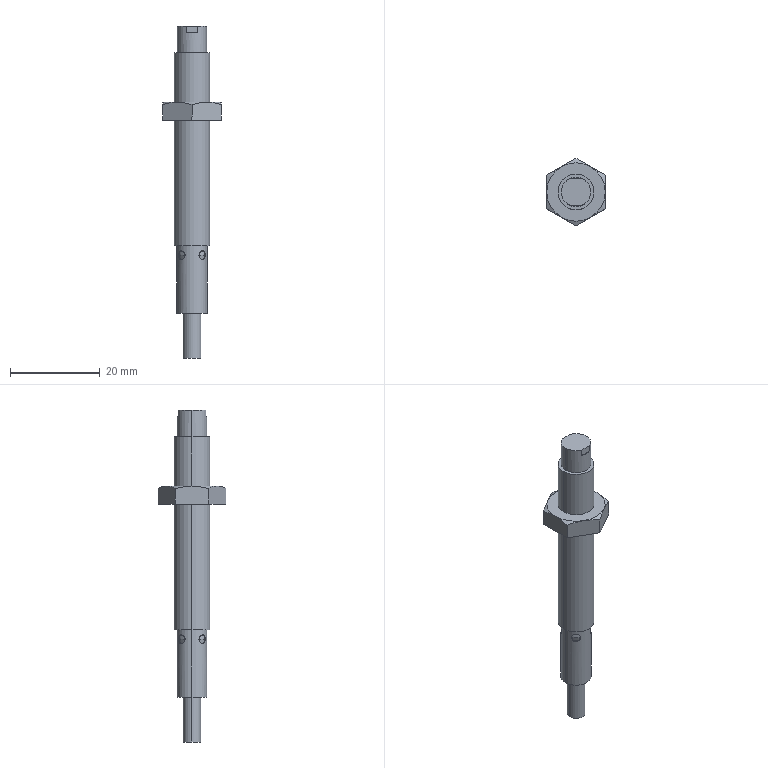Part | SolidWorks | features BaseBody 2 | 2 solids | 49 faces | box 13 x 15.011 x 74 mm | volume 3399 mm3 | cylinder 18 | plane 17 | sphere 8 | cone 6 | commonest cylinder face diameters 2 x8 8 x4 4 x2 6.6 x2 6.7 x2
STEP:
#1=CARTESIAN_POINT('',(4.,0.,-49.));
#2=VERTEX_POINT('',#1);
#3=CARTESIAN_POINT('',(-4.,0.,-49.));
#4=VERTEX_POINT('',#3);
#5=CARTESIAN_POINT('',(0.,0.,-49.));
#6=DIRECTION('',(0.,0.,1.));
#7=DIRECTION('',(1.,0.,0.));
#8=AXIS2_PLACEMENT_3D('',#5,#6,#7);
#9=CIRCLE('',#8,4.);
#10=EDGE_CURVE('',#2,#4,#9,.T.);
#11=ORIENTED_EDGE('',*,*,#10,.T.);
#12=CARTESIAN_POINT('',(-4.,0.,-6.));
#13=VERTEX_POINT('',#12);
#14=CARTESIAN_POINT('',(-4.,0.,22.148));
#15=DIRECTION('',(0.,0.,1.));
#16=VECTOR('',#15,1000.);
#17=LINE('',#14,#16);
#18=EDGE_CURVE('',#4,#13,#17,.T.);
#19=ORIENTED_EDGE('',*,*,#18,.T.);
#20=CARTESIAN_POINT('',(4.,0.,-6.));
#21=VERTEX_POINT('',#20);
#22=CARTESIAN_POINT('',(0.,0.,-6.));
#23=DIRECTION('',(0.,0.,-1.));
#24=DIRECTION('',(1.,0.,0.));
#25=AXIS2_PLACEMENT_3D('',#22,#23,#24);
#26=CIRCLE('',#25,4.);
#27=EDGE_CURVE('',#13,#21,#26,.T.);
#28=ORIENTED_EDGE('',*,*,#27,.T.);
#29=CARTESIAN_POINT('',(4.,0.,22.148));
#30=DIRECTION('',(0.,0.,1.));
#31=VECTOR('',#30,1000.);
#32=LINE('',#29,#31);
#33=EDGE_CURVE('',#2,#21,#32,.T.);
#34=ORIENTED_EDGE('',*,*,#33,.F.);
#35=EDGE_LOOP('',(#11,#19,#28,#34));
#36=FACE_OUTER_BOUND('',#35,.T.);
#37=CARTESIAN_POINT('',(0.,0.,22.148));
#38=DIRECTION('',(0.,0.,1.));
#39=DIRECTION('',(1.,0.,0.));
#40=AXIS2_PLACEMENT_3D('',#37,#38,#39);
#41=CYLINDRICAL_SURFACE('',#40,4.);
#42=ADVANCED_FACE('',(#36),#41,.T.);
#43=CARTESIAN_POINT('',(-3.3,0.,-6.));
#44=VERTEX_POINT('',#43);
#45=CARTESIAN_POINT('',(3.3,0.,-6.));
#46=VERTEX_POINT('',#45);
#47=CARTESIAN_POINT('',(0.,0.,-6.));
#48=DIRECTION('',(0.,0.,-1.));
#49=DIRECTION('',(1.,0.,0.));
#50=AXIS2_PLACEMENT_3D('',#47,#48,#49);
#51=CIRCLE('',#50,3.3);
#52=EDGE_CURVE('',#44,#46,#51,.T.);
#53=ORIENTED_EDGE('',*,*,#52,.F.);
#54=CARTESIAN_POINT('',(-3.3,0.,0.));
#55=VERTEX_POINT('',#54);
#56=CARTESIAN_POINT('',(-3.3,0.,5.792));
#57=DIRECTION('',(0.,0.,1.));
#58=VECTOR('',#57,1000.);
#59=LINE('',#56,#58);
#60=EDGE_CURVE('',#44,#55,#59,.T.);
#61=ORIENTED_EDGE('',*,*,#60,.T.);
#62=CARTESIAN_POINT('',(-1.26,3.05,0.));
#63=VERTEX_POINT('',#62);
#64=CARTESIAN_POINT('',(0.,0.,0.));
#65=DIRECTION('',(0.,0.,-1.));
#66=DIRECTION('',(1.,0.,0.));
#67=AXIS2_PLACEMENT_3D('',#64,#65,#66);
#68=CIRCLE('',#67,3.3);
#69=EDGE_CURVE('',#55,#63,#68,.T.);
#70=ORIENTED_EDGE('',*,*,#69,.T.);
#71=CARTESIAN_POINT('',(-1.26,3.05,-1.5));
#72=VERTEX_POINT('',#71);
#73=CARTESIAN_POINT('',(-1.26,3.05,0.));
#74=DIRECTION('',(0.,0.,-1.));
#75=VECTOR('',#74,1000.);
#76=LINE('',#73,#75);
#77=EDGE_CURVE('',#63,#72,#76,.T.);
#78=ORIENTED_EDGE('',*,*,#77,.T.);
#79=CARTESIAN_POINT('',(1.26,3.05,-1.5));
#80=VERTEX_POINT('',#79);
#81=CARTESIAN_POINT('',(0.,0.,-1.5));
#82=DIRECTION('',(0.,0.,-1.));
#83=DIRECTION('',(1.,0.,0.));
#84=AXIS2_PLACEMENT_3D('',#81,#82,#83);
#85=CIRCLE('',#84,3.3);
#86=EDGE_CURVE('',#72,#80,#85,.T.);
#87=ORIENTED_EDGE('',*,*,#86,.T.);
#88=CARTESIAN_POINT('',(1.26,3.05,0.));
#89=VERTEX_POINT('',#88);
#90=CARTESIAN_POINT('',(1.26,3.05,0.));
#91=DIRECTION('',(0.,0.,1.));
#92=VECTOR('',#91,1000.);
#93=LINE('',#90,#92);
#94=EDGE_CURVE('',#80,#89,#93,.T.);
#95=ORIENTED_EDGE('',*,*,#94,.T.);
#96=CARTESIAN_POINT('',(3.3,0.,0.));
#97=VERTEX_POINT('',#96);
#98=CARTESIAN_POINT('',(0.,0.,0.));
#99=DIRECTION('',(0.,0.,-1.));
#100=DIRECTION('',(1.,0.,0.));
#101=AXIS2_PLACEMENT_3D('',#98,#99,#100);
#102=CIRCLE('',#101,3.3);
#103=EDGE_CURVE('',#89,#97,#102,.T.);
#104=ORIENTED_EDGE('',*,*,#103,.T.);
#105=CARTESIAN_POINT('',(3.3,0.,5.792));
#106=DIRECTION('',(0.,0.,1.));
#107=VECTOR('',#106,1000.);
#108=LINE('',#105,#107);
#109=EDGE_CURVE('',#46,#97,#108,.T.);
#110=ORIENTED_EDGE('',*,*,#109,.F.);
#111=EDGE_LOOP('',(#53,#61,#70,#78,#87,#95,#104,#110));
#112=FACE_OUTER_BOUND('',#111,.T.);
#113=CARTESIAN_POINT('',(0.,0.,5.792));
#114=DIRECTION('',(0.,0.,1.));
#115=DIRECTION('',(1.,0.,0.));
#116=AXIS2_PLACEMENT_3D('',#113,#114,#115);
#117=CYLINDRICAL_SURFACE('',#116,3.3);
#118=ADVANCED_FACE('',(#112),#117,.T.);
#119=CARTESIAN_POINT('',(-1.554,2.968,-51.1));
#120=VERTEX_POINT('',#119);
#121=CARTESIAN_POINT('',(-2.968,1.554,-51.1));
#122=VERTEX_POINT('',#121);
#123=CARTESIAN_POINT('',(-1.554,2.968,-51.1));
#124=CARTESIAN_POINT('',(-1.554,2.968,-50.967));
#125=CARTESIAN_POINT('',(-1.578,2.955,-50.837));
#126=CARTESIAN_POINT('',(-1.67,2.905,-50.595));
#127=CARTESIAN_POINT('',(-1.737,2.866,-50.485));
#128=CARTESIAN_POINT('',(-1.894,2.765,-50.301));
#129=CARTESIAN_POINT('',(-1.987,2.7,-50.227));
#130=CARTESIAN_POINT('',(-2.176,2.55,-50.127));
#131=CARTESIAN_POINT('',(-2.275,2.462,-50.1));
#132=CARTESIAN_POINT('',(-2.461,2.277,-50.1));
#133=CARTESIAN_POINT('',(-2.548,2.178,-50.126));
#134=CARTESIAN_POINT('',(-2.7,1.986,-50.227));
#135=CARTESIAN_POINT('',(-2.764,1.895,-50.3));
#136=CARTESIAN_POINT('',(-2.918,1.657,-50.577));
#137=CARTESIAN_POINT('',(-2.968,1.554,-50.834));
#138=CARTESIAN_POINT('',(-2.968,1.554,-51.1));
#139=B_SPLINE_CURVE_WITH_KNOTS('',3,(#123,#124,#125,#126,#127,#128,#129,#130,#131,#132,#133,#134,#135,#136,#137,#138),.UNSPECIFIED.,.F.,.F.,(4,2,2,2,2,2,2,4),(0.003143,0.003536,0.003929,0.004322,0.004715,0.005108,0.005501,0.006286),.UNSPECIFIED.);
#140=EDGE_CURVE('',#120,#122,#139,.T.);
#141=ORIENTED_EDGE('',*,*,#140,.T.);
#142=CARTESIAN_POINT('',(-2.968,1.554,-51.1));
#143=CARTESIAN_POINT('',(-2.968,1.554,-51.233));
#144=CARTESIAN_POINT('',(-2.955,1.578,-51.363));
#145=CARTESIAN_POINT('',(-2.905,1.67,-51.605));
#146=CARTESIAN_POINT('',(-2.866,1.737,-51.715));
#147=CARTESIAN_POINT('',(-2.765,1.894,-51.899));
#148=CARTESIAN_POINT('',(-2.7,1.987,-51.973));
#149=CARTESIAN_POINT('',(-2.55,2.176,-52.073));
#150=CARTESIAN_POINT('',(-2.462,2.275,-52.1));
#151=CARTESIAN_POINT('',(-2.277,2.461,-52.1));
#152=CARTESIAN_POINT('',(-2.178,2.548,-52.074));
#153=CARTESIAN_POINT('',(-1.986,2.7,-51.973));
#154=CARTESIAN_POINT('',(-1.895,2.764,-51.9));
#155=CARTESIAN_POINT('',(-1.657,2.918,-51.623));
#156=CARTESIAN_POINT('',(-1.554,2.968,-51.366));
#157=CARTESIAN_POINT('',(-1.554,2.968,-51.1));
#158=B_SPLINE_CURVE_WITH_KNOTS('',3,(#142,#143,#144,#145,#146,#147,#148,#149,#150,#151,#152,#153,#154,#155,#156,#157),.UNSPECIFIED.,.F.,.F.,(4,2,2,2,2,2,2,4),(0.,0.0003929,0.0007858,0.001179,0.001572,0.001965,0.002357,0.003143),.UNSPECIFIED.);
#159=EDGE_CURVE('',#122,#120,#158,.T.);
#160=ORIENTED_EDGE('',*,*,#159,.T.);
#161=EDGE_LOOP('',(#141,#160));
#162=FACE_BOUND('',#161,.T.);
#163=CARTESIAN_POINT('',(2.968,1.554,-51.1));
#164=VERTEX_POINT('',#163);
#165=CARTESIAN_POINT('',(1.554,2.968,-51.1));
#166=VERTEX_POINT('',#165);
#167=CARTESIAN_POINT('',(2.968,1.554,-51.1));
#168=CARTESIAN_POINT('',(2.968,1.554,-50.967));
#169=CARTESIAN_POINT('',(2.955,1.578,-50.837));
#170=CARTESIAN_POINT('',(2.905,1.67,-50.595));
#171=CARTESIAN_POINT('',(2.866,1.737,-50.485));
#172=CARTESIAN_POINT('',(2.765,1.894,-50.301));
#173=CARTESIAN_POINT('',(2.7,1.987,-50.227));
#174=CARTESIAN_POINT('',(2.55,2.176,-50.127));
#175=CARTESIAN_POINT('',(2.462,2.275,-50.1));
#176=CARTESIAN_POINT('',(2.277,2.461,-50.1));
#177=CARTESIAN_POINT('',(2.178,2.548,-50.126));
#178=CARTESIAN_POINT('',(1.986,2.7,-50.227));
#179=CARTESIAN_POINT('',(1.895,2.764,-50.3));
#180=CARTESIAN_POINT('',(1.657,2.918,-50.577));
#181=CARTESIAN_POINT('',(1.554,2.968,-50.834));
#182=CARTESIAN_POINT('',(1.554,2.968,-51.1));
#183=B_SPLINE_CURVE_WITH_KNOTS('',3,(#167,#168,#169,#170,#171,#172,#173,#174,#175,#176,#177,#178,#179,#180,#181,#182),.UNSPECIFIED.,.F.,.F.,(4,2,2,2,2,2,2,4),(0.003143,0.003536,0.003929,0.004322,0.004715,0.005108,0.005501,0.006286),.UNSPECIFIED.);
#184=EDGE_CURVE('',#164,#166,#183,.T.);
#185=ORIENTED_EDGE('',*,*,#184,.T.);
#186=CARTESIAN_POINT('',(1.554,2.968,-51.1));
#187=CARTESIAN_POINT('',(1.554,2.968,-51.233));
#188=CARTESIAN_POINT('',(1.578,2.955,-51.363));
#189=CARTESIAN_POINT('',(1.67,2.905,-51.605));
#190=CARTESIAN_POINT('',(1.737,2.866,-51.715));
#191=CARTESIAN_POINT('',(1.894,2.765,-51.899));
#192=CARTESIAN_POINT('',(1.987,2.7,-51.973));
#193=CARTESIAN_POINT('',(2.176,2.55,-52.073));
#194=CARTESIAN_POINT('',(2.275,2.462,-52.1));
#195=CARTESIAN_POINT('',(2.461,2.277,-52.1));
#196=CARTESIAN_POINT('',(2.548,2.178,-52.074));
#197=CARTESIAN_POINT('',(2.7,1.986,-51.973));
#198=CARTESIAN_POINT('',(2.764,1.895,-51.9));
#199=CARTESIAN_POINT('',(2.918,1.657,-51.623));
#200=CARTESIAN_POINT('',(2.968,1.554,-51.366));
#201=CARTESIAN_POINT('',(2.968,1.554,-51.1));
#202=B_SPLINE_CURVE_WITH_KNOTS('',3,(#186,#187,#188,#189,#190,#191,#192,#193,#194,#195,#196,#197,#198,#199,#200,#201),.UNSPECIFIED.,.F.,.F.,(4,2,2,2,2,2,2,4),(0.,0.0003929,0.0007858,0.001179,0.001572,0.001965,0.002357,0.003143),.UNSPECIFIED.);
#203=EDGE_CURVE('',#166,#164,#202,.T.);
#204=ORIENTED_EDGE('',*,*,#203,.T.);
#205=EDGE_LOOP('',(#185,#204));
#206=FACE_BOUND('',#205,.T.);
#207=CARTESIAN_POINT('',(3.35,0.,-64.));
#208=VERTEX_POINT('',#207);
#209=CARTESIAN_POINT('',(-3.35,0.,-64.));
#210=VERTEX_POINT('',#209);
#211=CARTESIAN_POINT('',(0.,0.,-64.));
#212=DIRECTION('',(0.,0.,1.));
#213=DIRECTION('',(1.,0.,0.));
#214=AXIS2_PLACEMENT_3D('',#211,#212,#213);
#215=CIRCLE('',#214,3.35);
#216=EDGE_CURVE('',#208,#210,#215,.T.);
#217=ORIENTED_EDGE('',*,*,#216,.T.);
#218=CARTESIAN_POINT('',(-3.35,0.,-49.));
#219=VERTEX_POINT('',#218);
#220=CARTESIAN_POINT('',(-3.35,0.,22.148));
#221=DIRECTION('',(0.,0.,1.));
#222=VECTOR('',#221,1000.);
#223=LINE('',#220,#222);
#224=EDGE_CURVE('',#210,#219,#223,.T.);
#225=ORIENTED_EDGE('',*,*,#224,.T.);
#226=CARTESIAN_POINT('',(3.35,0.,-49.));
#227=VERTEX_POINT('',#226);
#228=CARTESIAN_POINT('',(0.,0.,-49.));
#229=DIRECTION('',(0.,0.,1.));
#230=DIRECTION('',(1.,0.,0.));
#231=AXIS2_PLACEMENT_3D('',#228,#229,#230);
#232=CIRCLE('',#231,3.35);
#233=EDGE_CURVE('',#227,#219,#232,.T.);
#234=ORIENTED_EDGE('',*,*,#233,.F.);
#235=CARTESIAN_POINT('',(3.35,0.,22.148));
#236=DIRECTION('',(0.,0.,1.));
#237=VECTOR('',#236,1000.);
#238=LINE('',#235,#237);
#239=EDGE_CURVE('',#208,#227,#238,.T.);
#240=ORIENTED_EDGE('',*,*,#239,.F.);
#241=EDGE_LOOP('',(#217,#225,#234,#240));
#242=FACE_OUTER_BOUND('',#241,.T.);
#243=CARTESIAN_POINT('',(0.,0.,22.148));
#244=DIRECTION('',(0.,0.,1.));
#245=DIRECTION('',(1.,0.,0.));
#246=AXIS2_PLACEMENT_3D('',#243,#244,#245);
#247=CYLINDRICAL_SURFACE('',#246,3.35);
#248=ADVANCED_FACE('',(#162,#206,#242),#247,.T.);
#249=CARTESIAN_POINT('',(-1.554,-2.968,-51.1));
#250=VERTEX_POINT('',#249);
#251=CARTESIAN_POINT('',(-2.968,-1.554,-51.1));
#252=VERTEX_POINT('',#251);
#253=CARTESIAN_POINT('',(-1.554,-2.968,-51.1));
#254=CARTESIAN_POINT('',(-1.554,-2.968,-51.233));
#255=CARTESIAN_POINT('',(-1.578,-2.955,-51.363));
#256=CARTESIAN_POINT('',(-1.67,-2.905,-51.605));
#257=CARTESIAN_POINT('',(-1.737,-2.866,-51.715));
#258=CARTESIAN_POINT('',(-1.894,-2.765,-51.899));
#259=CARTESIAN_POINT('',(-1.987,-2.7,-51.973));
#260=CARTESIAN_POINT('',(-2.176,-2.55,-52.073));
#261=CARTESIAN_POINT('',(-2.275,-2.462,-52.1));
#262=CARTESIAN_POINT('',(-2.461,-2.277,-52.1));
#263=CARTESIAN_POINT('',(-2.548,-2.178,-52.074));
#264=CARTESIAN_POINT('',(-2.7,-1.986,-51.973));
#265=CARTESIAN_POINT('',(-2.764,-1.895,-51.9));
#266=CARTESIAN_POINT('',(-2.918,-1.657,-51.623));
#267=CARTESIAN_POINT('',(-2.968,-1.554,-51.366));
#268=CARTESIAN_POINT('',(-2.968,-1.554,-51.1));
#269=B_SPLINE_CURVE_WITH_KNOTS('',3,(#253,#254,#255,#256,#257,#258,#259,#260,#261,#262,#263,#264,#265,#266,#267,#268),.UNSPECIFIED.,.F.,.F.,(4,2,2,2,2,2,2,4),(0.,0.0003929,0.0007858,0.001179,0.001572,0.001965,0.002357,0.003143),.UNSPECIFIED.);
#270=EDGE_CURVE('',#250,#252,#269,.T.);
#271=ORIENTED_EDGE('',*,*,#270,.F.);
#272=CARTESIAN_POINT('',(-1.405,-2.819,-51.1));
#273=VERTEX_POINT('',#272);
#274=CARTESIAN_POINT('',(0.7071,-0.7071,-51.1));
#275=DIRECTION('',(0.7071,0.7071,0.));
#276=VECTOR('',#275,1000.);
#277=LINE('',#274,#276);
#278=EDGE_CURVE('',#250,#273,#277,.T.);
#279=ORIENTED_EDGE('',*,*,#278,.T.);
#280=CARTESIAN_POINT('',(-2.819,-1.405,-51.1));
#281=VERTEX_POINT('',#280);
#282=CARTESIAN_POINT('',(-2.112,-2.112,-51.1));
#283=DIRECTION('',(-0.7071,-0.7071,0.));
#284=DIRECTION('',(-0.7071,0.7071,0.));
#285=AXIS2_PLACEMENT_3D('',#282,#283,#284);
#286=CIRCLE('',#285,1.);
#287=EDGE_CURVE('',#281,#273,#286,.T.);
#288=ORIENTED_EDGE('',*,*,#287,.F.);
#289=CARTESIAN_POINT('',(-0.7071,0.7071,-51.1));
#290=DIRECTION('',(0.7071,0.7071,0.));
#291=VECTOR('',#290,1000.);
#292=LINE('',#289,#291);
#293=EDGE_CURVE('',#252,#281,#292,.T.);
#294=ORIENTED_EDGE('',*,*,#293,.F.);
#295=EDGE_LOOP('',(#271,#279,#288,#294));
#296=FACE_OUTER_BOUND('',#295,.T.);
#297=CARTESIAN_POINT('',(0.,0.,-51.1));
#298=DIRECTION('',(0.7071,0.7071,0.));
#299=DIRECTION('',(-0.7071,0.7071,0.));
#300=AXIS2_PLACEMENT_3D('',#297,#298,#299);
#301=CYLINDRICAL_SURFACE('',#300,1.);
#302=ADVANCED_FACE('',(#296),#301,.F.);
#303=CARTESIAN_POINT('',(2.968,-1.554,-51.1));
#304=VERTEX_POINT('',#303);
#305=CARTESIAN_POINT('',(1.554,-2.968,-51.1));
#306=VERTEX_POINT('',#305);
#307=CARTESIAN_POINT('',(2.968,-1.554,-51.1));
#308=CARTESIAN_POINT('',(2.968,-1.554,-51.233));
#309=CARTESIAN_POINT('',(2.955,-1.578,-51.363));
#310=CARTESIAN_POINT('',(2.905,-1.67,-51.605));
#311=CARTESIAN_POINT('',(2.866,-1.737,-51.715));
#312=CARTESIAN_POINT('',(2.765,-1.894,-51.899));
#313=CARTESIAN_POINT('',(2.7,-1.987,-51.973));
#314=CARTESIAN_POINT('',(2.55,-2.176,-52.073));
#315=CARTESIAN_POINT('',(2.462,-2.275,-52.1));
#316=CARTESIAN_POINT('',(2.277,-2.461,-52.1));
#317=CARTESIAN_POINT('',(2.178,-2.548,-52.074));
#318=CARTESIAN_POINT('',(1.986,-2.7,-51.973));
#319=CARTESIAN_POINT('',(1.895,-2.764,-51.9));
#320=CARTESIAN_POINT('',(1.657,-2.918,-51.623));
#321=CARTESIAN_POINT('',(1.554,-2.968,-51.366));
#322=CARTESIAN_POINT('',(1.554,-2.968,-51.1));
#323=B_SPLINE_CURVE_WITH_KNOTS('',3,(#307,#308,#309,#310,#311,#312,#313,#314,#315,#316,#317,#318,#319,#320,#321,#322),.UNSPECIFIED.,.F.,.F.,(4,2,2,2,2,2,2,4),(0.,0.0003929,0.0007858,0.001179,0.001572,0.001965,0.002357,0.003143),.UNSPECIFIED.);
#324=EDGE_CURVE('',#304,#306,#323,.T.);
#325=ORIENTED_EDGE('',*,*,#324,.F.);
#326=CARTESIAN_POINT('',(2.819,-1.405,-51.1));
#327=VERTEX_POINT('',#326);
#328=CARTESIAN_POINT('',(0.7071,0.7071,-51.1));
#329=DIRECTION('',(-0.7071,0.7071,0.));
#330=VECTOR('',#329,1000.);
#331=LINE('',#328,#330);
#332=EDGE_CURVE('',#304,#327,#331,.T.);
#333=ORIENTED_EDGE('',*,*,#332,.T.);
#334=CARTESIAN_POINT('',(1.405,-2.819,-51.1));
#335=VERTEX_POINT('',#334);
#336=CARTESIAN_POINT('',(2.112,-2.112,-51.1));
#337=DIRECTION('',(0.7071,-0.7071,0.));
#338=DIRECTION('',(-0.7071,-0.7071,0.));
#339=AXIS2_PLACEMENT_3D('',#336,#337,#338);
#340=CIRCLE('',#339,1.);
#341=EDGE_CURVE('',#335,#327,#340,.T.);
#342=ORIENTED_EDGE('',*,*,#341,.F.);
#343=CARTESIAN_POINT('',(-0.7071,-0.7071,-51.1));
#344=DIRECTION('',(-0.7071,0.7071,0.));
#345=VECTOR('',#344,1000.);
#346=LINE('',#343,#345);
#347=EDGE_CURVE('',#306,#335,#346,.T.);
#348=ORIENTED_EDGE('',*,*,#347,.F.);
#349=EDGE_LOOP('',(#325,#333,#342,#348));
#350=FACE_OUTER_BOUND('',#349,.T.);
#351=CARTESIAN_POINT('',(0.,0.,-51.1));
#352=DIRECTION('',(-0.7071,0.7071,0.));
#353=DIRECTION('',(-0.7071,-0.7071,0.));
#354=AXIS2_PLACEMENT_3D('',#351,#352,#353);
#355=CYLINDRICAL_SURFACE('',#354,1.);
#356=ADVANCED_FACE('',(#350),#355,.F.);
#357=ORIENTED_EDGE('',*,*,#203,.F.);
#358=CARTESIAN_POINT('',(1.405,2.819,-51.1));
#359=VERTEX_POINT('',#358);
#360=CARTESIAN_POINT('',(-0.7071,0.7071,-51.1));
#361=DIRECTION('',(-0.7071,-0.7071,0.));
#362=VECTOR('',#361,1000.);
#363=LINE('',#360,#362);
#364=EDGE_CURVE('',#166,#359,#363,.T.);
#365=ORIENTED_EDGE('',*,*,#364,.T.);
#366=CARTESIAN_POINT('',(2.819,1.405,-51.1));
#367=VERTEX_POINT('',#366);
#368=CARTESIAN_POINT('',(2.112,2.112,-51.1));
#369=DIRECTION('',(0.7071,0.7071,0.));
#370=DIRECTION('',(0.7071,-0.7071,0.));
#371=AXIS2_PLACEMENT_3D('',#368,#369,#370);
#372=CIRCLE('',#371,1.);
#373=EDGE_CURVE('',#367,#359,#372,.T.);
#374=ORIENTED_EDGE('',*,*,#373,.F.);
#375=CARTESIAN_POINT('',(0.7071,-0.7071,-51.1));
#376=DIRECTION('',(-0.7071,-0.7071,0.));
#377=VECTOR('',#376,1000.);
#378=LINE('',#375,#377);
#379=EDGE_CURVE('',#164,#367,#378,.T.);
#380=ORIENTED_EDGE('',*,*,#379,.F.);
#381=EDGE_LOOP('',(#357,#365,#374,#380));
#382=FACE_OUTER_BOUND('',#381,.T.);
#383=CARTESIAN_POINT('',(0.,0.,-51.1));
#384=DIRECTION('',(-0.7071,-0.7071,0.));
#385=DIRECTION('',(0.7071,-0.7071,0.));
#386=AXIS2_PLACEMENT_3D('',#383,#384,#385);
#387=CYLINDRICAL_SURFACE('',#386,1.);
#388=ADVANCED_FACE('',(#382),#387,.F.);
#389=ORIENTED_EDGE('',*,*,#159,.F.);
#390=CARTESIAN_POINT('',(-2.819,1.405,-51.1));
#391=VERTEX_POINT('',#390);
#392=CARTESIAN_POINT('',(-0.7071,-0.7071,-51.1));
#393=DIRECTION('',(0.7071,-0.7071,0.));
#394=VECTOR('',#393,1000.);
#395=LINE('',#392,#394);
#396=EDGE_CURVE('',#122,#391,#395,.T.);
#397=ORIENTED_EDGE('',*,*,#396,.T.);
#398=CARTESIAN_POINT('',(-1.405,2.819,-51.1));
#399=VERTEX_POINT('',#398);
#400=CARTESIAN_POINT('',(-2.112,2.112,-51.1));
#401=DIRECTION('',(-0.7071,0.7071,0.));
#402=DIRECTION('',(0.7071,0.7071,0.));
#403=AXIS2_PLACEMENT_3D('',#400,#401,#402);
#404=CIRCLE('',#403,1.);
#405=EDGE_CURVE('',#399,#391,#404,.T.);
#406=ORIENTED_EDGE('',*,*,#405,.F.);
#407=CARTESIAN_POINT('',(0.7071,0.7071,-51.1));
#408=DIRECTION('',(0.7071,-0.7071,0.));
#409=VECTOR('',#408,1000.);
#410=LINE('',#407,#409);
#411=EDGE_CURVE('',#120,#399,#410,.T.);
#412=ORIENTED_EDGE('',*,*,#411,.F.);
#413=EDGE_LOOP('',(#389,#397,#406,#412));
#414=FACE_OUTER_BOUND('',#413,.T.);
#415=CARTESIAN_POINT('',(0.,0.,-51.1));
#416=DIRECTION('',(0.7071,-0.7071,0.));
#417=DIRECTION('',(0.7071,0.7071,0.));
#418=AXIS2_PLACEMENT_3D('',#415,#416,#417);
#419=CYLINDRICAL_SURFACE('',#418,1.);
#420=ADVANCED_FACE('',(#414),#419,.F.);
#421=CARTESIAN_POINT('',(-2.112,-2.112,-51.1));
#422=DIRECTION('',(-0.7071,-0.7071,0.));
#423=DIRECTION('',(-0.7071,0.7071,0.));
#424=AXIS2_PLACEMENT_3D('',#421,#422,#423);
#425=CIRCLE('',#424,1.);
#426=EDGE_CURVE('',#273,#281,#425,.T.);
#427=ORIENTED_EDGE('',*,*,#426,.T.);
#428=CARTESIAN_POINT('',(0.,0.,-51.1));
#429=DIRECTION('',(0.,0.,1.));
#430=DIRECTION('',(1.,0.,0.));
#431=AXIS2_PLACEMENT_3D('',#428,#429,#430);
#432=CIRCLE('',#431,3.15);
#433=EDGE_CURVE('',#281,#273,#432,.T.);
#434=ORIENTED_EDGE('',*,*,#433,.T.);
#435=EDGE_LOOP('',(#427,#434));
#436=FACE_OUTER_BOUND('',#435,.T.);
#437=CARTESIAN_POINT('',(0.,0.,-51.1));
#438=DIRECTION('',(0.,0.,-1.));
#439=DIRECTION('',(-0.7071,-0.7071,0.));
#440=AXIS2_PLACEMENT_3D('',#437,#438,#439);
#441=SPHERICAL_SURFACE('',#440,3.15);
#442=ADVANCED_FACE('',(#436),#441,.T.);
#443=CARTESIAN_POINT('',(2.112,-2.112,-51.1));
#444=DIRECTION('',(0.7071,-0.7071,0.));
#445=DIRECTION('',(-0.7071,-0.7071,0.));
#446=AXIS2_PLACEMENT_3D('',#443,#444,#445);
#447=CIRCLE('',#446,1.);
#448=EDGE_CURVE('',#327,#335,#447,.T.);
#449=ORIENTED_EDGE('',*,*,#448,.T.);
#450=CARTESIAN_POINT('',(0.,0.,-51.1));
#451=DIRECTION('',(0.,0.,1.));
#452=DIRECTION('',(1.,0.,0.));
#453=AXIS2_PLACEMENT_3D('',#450,#451,#452);
#454=CIRCLE('',#453,3.15);
#455=EDGE_CURVE('',#335,#327,#454,.T.);
#456=ORIENTED_EDGE('',*,*,#455,.T.);
#457=EDGE_LOOP('',(#449,#456));
#458=FACE_OUTER_BOUND('',#457,.T.);
#459=CARTESIAN_POINT('',(0.,0.,-51.1));
#460=DIRECTION('',(0.,0.,-1.));
#461=DIRECTION('',(0.7071,-0.7071,0.));
#462=AXIS2_PLACEMENT_3D('',#459,#460,#461);
#463=SPHERICAL_SURFACE('',#462,3.15);
#464=ADVANCED_FACE('',(#458),#463,.T.);
#465=CARTESIAN_POINT('',(2.,0.,-74.));
#466=VERTEX_POINT('',#465);
#467=CARTESIAN_POINT('',(-2.,0.,-74.));
#468=VERTEX_POINT('',#467);
#469=CARTESIAN_POINT('',(0.,0.,-74.));
#470=DIRECTION('',(0.,0.,1.));
#471=DIRECTION('',(1.,0.,0.));
#472=AXIS2_PLACEMENT_3D('',#469,#470,#471);
#473=CIRCLE('',#472,2.);
#474=EDGE_CURVE('',#466,#468,#473,.T.);
#475=ORIENTED_EDGE('',*,*,#474,.T.);
#476=CARTESIAN_POINT('',(-2.,0.,-64.));
#477=VERTEX_POINT('',#476);
#478=CARTESIAN_POINT('',(-2.,0.,0.));
#479=DIRECTION('',(0.,0.,1.));
#480=VECTOR('',#479,1000.);
#481=LINE('',#478,#480);
#482=EDGE_CURVE('',#468,#477,#481,.T.);
#483=ORIENTED_EDGE('',*,*,#482,.T.);
#484=CARTESIAN_POINT('',(2.,0.,-64.));
#485=VERTEX_POINT('',#484);
#486=CARTESIAN_POINT('',(0.,0.,-64.));
#487=DIRECTION('',(0.,0.,1.));
#488=DIRECTION('',(1.,0.,0.));
#489=AXIS2_PLACEMENT_3D('',#486,#487,#488);
#490=CIRCLE('',#489,2.);
#491=EDGE_CURVE('',#485,#477,#490,.T.);
#492=ORIENTED_EDGE('',*,*,#491,.F.);
#493=CARTESIAN_POINT('',(2.,0.,0.));
#494=DIRECTION('',(0.,0.,1.));
#495=VECTOR('',#494,1000.);
#496=LINE('',#493,#495);
#497=EDGE_CURVE('',#466,#485,#496,.T.);
#498=ORIENTED_EDGE('',*,*,#497,.F.);
#499=EDGE_LOOP('',(#475,#483,#492,#498));
#500=FACE_OUTER_BOUND('',#499,.T.);
#501=CARTESIAN_POINT('',(0.,0.,0.));
#502=DIRECTION('',(0.,0.,1.));
#503=DIRECTION('',(1.,0.,0.));
#504=AXIS2_PLACEMENT_3D('',#501,#502,#503);
#505=CYLINDRICAL_SURFACE('',#504,2.);
#506=ADVANCED_FACE('',(#500),#505,.T.);
#507=CARTESIAN_POINT('',(2.112,2.112,-51.1));
#508=DIRECTION('',(0.7071,0.7071,0.));
#509=DIRECTION('',(0.7071,-0.7071,0.));
#510=AXIS2_PLACEMENT_3D('',#507,#508,#509);
#511=CIRCLE('',#510,1.);
#512=EDGE_CURVE('',#359,#367,#511,.T.);
#513=ORIENTED_EDGE('',*,*,#512,.T.);
#514=CARTESIAN_POINT('',(0.,0.,-51.1));
#515=DIRECTION('',(0.,0.,1.));
#516=DIRECTION('',(1.,0.,0.));
#517=AXIS2_PLACEMENT_3D('',#514,#515,#516);
#518=CIRCLE('',#517,3.15);
#519=EDGE_CURVE('',#367,#359,#518,.T.);
#520=ORIENTED_EDGE('',*,*,#519,.T.);
#521=EDGE_LOOP('',(#513,#520));
#522=FACE_OUTER_BOUND('',#521,.T.);
#523=CARTESIAN_POINT('',(0.,0.,-51.1));
#524=DIRECTION('',(0.,0.,-1.));
#525=DIRECTION('',(0.7071,0.7071,0.));
#526=AXIS2_PLACEMENT_3D('',#523,#524,#525);
#527=SPHERICAL_SURFACE('',#526,3.15);
#528=ADVANCED_FACE('',(#522),#527,.T.);
#529=CARTESIAN_POINT('',(-2.112,2.112,-51.1));
#530=DIRECTION('',(-0.7071,0.7071,0.));
#531=DIRECTION('',(0.7071,0.7071,0.));
#532=AXIS2_PLACEMENT_3D('',#529,#530,#531);
#533=CIRCLE('',#532,1.);
#534=EDGE_CURVE('',#391,#399,#533,.T.);
#535=ORIENTED_EDGE('',*,*,#534,.T.);
#536=CARTESIAN_POINT('',(0.,0.,-51.1));
#537=DIRECTION('',(0.,0.,1.));
#538=DIRECTION('',(0.,-1.,0.));
#539=AXIS2_PLACEMENT_3D('',#536,#537,#538);
#540=CIRCLE('',#539,3.15);
#541=EDGE_CURVE('',#399,#391,#540,.T.);
#542=ORIENTED_EDGE('',*,*,#541,.T.);
#543=EDGE_LOOP('',(#535,#542));
#544=FACE_OUTER_BOUND('',#543,.T.);
#545=CARTESIAN_POINT('',(0.,0.,-51.1));
#546=DIRECTION('',(0.,0.,-1.));
#547=DIRECTION('',(-0.7071,0.7071,0.));
#548=AXIS2_PLACEMENT_3D('',#545,#546,#547);
#549=SPHERICAL_SURFACE('',#548,3.15);
#550=ADVANCED_FACE('',(#544),#549,.T.);
#551=ORIENTED_EDGE('',*,*,#18,.F.);
#552=CARTESIAN_POINT('',(0.,0.,-49.));
#553=DIRECTION('',(0.,0.,1.));
#554=DIRECTION('',(1.,0.,0.));
#555=AXIS2_PLACEMENT_3D('',#552,#553,#554);
#556=CIRCLE('',#555,4.);
#557=EDGE_CURVE('',#4,#2,#556,.T.);
#558=ORIENTED_EDGE('',*,*,#557,.T.);
#559=ORIENTED_EDGE('',*,*,#33,.T.);
#560=CARTESIAN_POINT('',(0.,0.,-6.));
#561=DIRECTION('',(0.,0.,-1.));
#562=DIRECTION('',(1.,0.,0.));
#563=AXIS2_PLACEMENT_3D('',#560,#561,#562);
#564=CIRCLE('',#563,4.);
#565=EDGE_CURVE('',#21,#13,#564,.T.);
#566=ORIENTED_EDGE('',*,*,#565,.T.);
#567=EDGE_LOOP('',(#551,#558,#559,#566));
#568=FACE_OUTER_BOUND('',#567,.T.);
#569=CARTESIAN_POINT('',(0.,0.,22.148));
#570=DIRECTION('',(0.,0.,1.));
#571=DIRECTION('',(1.,0.,0.));
#572=AXIS2_PLACEMENT_3D('',#569,#570,#571);
#573=CYLINDRICAL_SURFACE('',#572,4.);
#574=ADVANCED_FACE('',(#568),#573,.T.);
#575=ORIENTED_EDGE('',*,*,#565,.F.);
#576=ORIENTED_EDGE('',*,*,#27,.F.);
#577=EDGE_LOOP('',(#575,#576));
#578=FACE_OUTER_BOUND('',#577,.T.);
#579=CARTESIAN_POINT('',(0.,0.,-6.));
#580=DIRECTION('',(0.,0.,-1.));
#581=DIRECTION('',(1.,0.,0.));
#582=AXIS2_PLACEMENT_3D('',#579,#580,#581);
#583=CIRCLE('',#582,3.3);
#584=EDGE_CURVE('',#46,#44,#583,.T.);
#585=ORIENTED_EDGE('',*,*,#584,.T.);
#586=ORIENTED_EDGE('',*,*,#52,.T.);
#587=EDGE_LOOP('',(#585,#586));
#588=FACE_BOUND('',#587,.T.);
#589=CARTESIAN_POINT('',(0.,0.,-6.));
#590=DIRECTION('',(0.,0.,1.));
#591=DIRECTION('',(1.,0.,0.));
#592=AXIS2_PLACEMENT_3D('',#589,#590,#591);
#593=PLANE('',#592);
#594=ADVANCED_FACE('',(#578,#588),#593,.T.);
#595=ORIENTED_EDGE('',*,*,#233,.T.);
#596=CARTESIAN_POINT('',(0.,0.,-49.));
#597=DIRECTION('',(0.,0.,1.));
#598=DIRECTION('',(1.,0.,0.));
#599=AXIS2_PLACEMENT_3D('',#596,#597,#598);
#600=CIRCLE('',#599,3.35);
#601=EDGE_CURVE('',#219,#227,#600,.T.);
#602=ORIENTED_EDGE('',*,*,#601,.T.);
#603=EDGE_LOOP('',(#595,#602));
#604=FACE_BOUND('',#603,.T.);
#605=ORIENTED_EDGE('',*,*,#10,.F.);
#606=ORIENTED_EDGE('',*,*,#557,.F.);
#607=EDGE_LOOP('',(#605,#606));
#608=FACE_OUTER_BOUND('',#607,.T.);
#609=CARTESIAN_POINT('',(0.,0.,-49.));
#610=DIRECTION('',(0.,0.,-1.));
#611=DIRECTION('',(-1.,0.,0.));
#612=AXIS2_PLACEMENT_3D('',#609,#610,#611);
#613=PLANE('',#612);
#614=ADVANCED_FACE('',(#604,#608),#613,.T.);
#615=ORIENTED_EDGE('',*,*,#60,.F.);
#616=ORIENTED_EDGE('',*,*,#584,.F.);
#617=ORIENTED_EDGE('',*,*,#109,.T.);
#618=CARTESIAN_POINT('',(1.26,-3.05,0.));
#619=VERTEX_POINT('',#618);
#620=CARTESIAN_POINT('',(0.,0.,0.));
#621=DIRECTION('',(0.,0.,-1.));
#622=DIRECTION('',(1.,0.,0.));
#623=AXIS2_PLACEMENT_3D('',#620,#621,#622);
#624=CIRCLE('',#623,3.3);
#625=EDGE_CURVE('',#97,#619,#624,.T.);
#626=ORIENTED_EDGE('',*,*,#625,.T.);
#627=CARTESIAN_POINT('',(1.26,-3.05,-1.5));
#628=VERTEX_POINT('',#627);
#629=CARTESIAN_POINT('',(1.26,-3.05,0.));
#630=DIRECTION('',(0.,0.,-1.));
#631=VECTOR('',#630,1000.);
#632=LINE('',#629,#631);
#633=EDGE_CURVE('',#619,#628,#632,.T.);
#634=ORIENTED_EDGE('',*,*,#633,.T.);
#635=CARTESIAN_POINT('',(-1.26,-3.05,-1.5));
#636=VERTEX_POINT('',#635);
#637=CARTESIAN_POINT('',(0.,0.,-1.5));
#638=DIRECTION('',(0.,0.,-1.));
#639=DIRECTION('',(1.,0.,0.));
#640=AXIS2_PLACEMENT_3D('',#637,#638,#639);
#641=CIRCLE('',#640,3.3);
#642=EDGE_CURVE('',#628,#636,#641,.T.);
#643=ORIENTED_EDGE('',*,*,#642,.T.);
#644=CARTESIAN_POINT('',(-1.26,-3.05,0.));
#645=VERTEX_POINT('',#644);
#646=CARTESIAN_POINT('',(-1.26,-3.05,0.));
#647=DIRECTION('',(0.,0.,1.));
#648=VECTOR('',#647,1000.);
#649=LINE('',#646,#648);
#650=EDGE_CURVE('',#636,#645,#649,.T.);
#651=ORIENTED_EDGE('',*,*,#650,.T.);
#652=CARTESIAN_POINT('',(0.,0.,0.));
#653=DIRECTION('',(0.,0.,-1.));
#654=DIRECTION('',(1.,0.,0.));
#655=AXIS2_PLACEMENT_3D('',#652,#653,#654);
#656=CIRCLE('',#655,3.3);
#657=EDGE_CURVE('',#645,#55,#656,.T.);
#658=ORIENTED_EDGE('',*,*,#657,.T.);
#659=EDGE_LOOP('',(#615,#616,#617,#626,#634,#643,#651,#658));
#660=FACE_OUTER_BOUND('',#659,.T.);
#661=CARTESIAN_POINT('',(0.,0.,5.792));
#662=DIRECTION('',(0.,0.,1.));
#663=DIRECTION('',(1.,0.,0.));
#664=AXIS2_PLACEMENT_3D('',#661,#662,#663);
#665=CYLINDRICAL_SURFACE('',#664,3.3);
#666=ADVANCED_FACE('',(#660),#665,.T.);
#667=ORIENTED_EDGE('',*,*,#224,.F.);
#668=CARTESIAN_POINT('',(0.,0.,-64.));
#669=DIRECTION('',(0.,0.,1.));
#670=DIRECTION('',(1.,0.,0.));
#671=AXIS2_PLACEMENT_3D('',#668,#669,#670);
#672=CIRCLE('',#671,3.35);
#673=EDGE_CURVE('',#210,#208,#672,.T.);
#674=ORIENTED_EDGE('',*,*,#673,.T.);
#675=ORIENTED_EDGE('',*,*,#239,.T.);
#676=ORIENTED_EDGE('',*,*,#601,.F.);
#677=EDGE_LOOP('',(#667,#674,#675,#676));
#678=FACE_OUTER_BOUND('',#677,.T.);
#679=CARTESIAN_POINT('',(-2.968,-1.554,-51.1));
#680=CARTESIAN_POINT('',(-2.968,-1.554,-50.967));
#681=CARTESIAN_POINT('',(-2.955,-1.578,-50.837));
#682=CARTESIAN_POINT('',(-2.905,-1.67,-50.595));
#683=CARTESIAN_POINT('',(-2.866,-1.737,-50.485));
#684=CARTESIAN_POINT('',(-2.765,-1.894,-50.301));
#685=CARTESIAN_POINT('',(-2.7,-1.987,-50.227));
#686=CARTESIAN_POINT('',(-2.55,-2.176,-50.127));
#687=CARTESIAN_POINT('',(-2.462,-2.275,-50.1));
#688=CARTESIAN_POINT('',(-2.277,-2.461,-50.1));
#689=CARTESIAN_POINT('',(-2.178,-2.548,-50.126));
#690=CARTESIAN_POINT('',(-1.986,-2.7,-50.227));
#691=CARTESIAN_POINT('',(-1.895,-2.764,-50.3));
#692=CARTESIAN_POINT('',(-1.657,-2.918,-50.577));
#693=CARTESIAN_POINT('',(-1.554,-2.968,-50.834));
#694=CARTESIAN_POINT('',(-1.554,-2.968,-51.1));
#695=B_SPLINE_CURVE_WITH_KNOTS('',3,(#679,#680,#681,#682,#683,#684,#685,#686,#687,#688,#689,#690,#691,#692,#693,#694),.UNSPECIFIED.,.F.,.F.,(4,2,2,2,2,2,2,4),(0.003143,0.003536,0.003929,0.004322,0.004715,0.005108,0.005501,0.006286),.UNSPECIFIED.);
#696=EDGE_CURVE('',#252,#250,#695,.T.);
#697=ORIENTED_EDGE('',*,*,#696,.T.);
#698=ORIENTED_EDGE('',*,*,#270,.T.);
#699=EDGE_LOOP('',(#697,#698));
#700=FACE_BOUND('',#699,.T.);
#701=CARTESIAN_POINT('',(1.554,-2.968,-51.1));
#702=CARTESIAN_POINT('',(1.554,-2.968,-50.967));
#703=CARTESIAN_POINT('',(1.578,-2.955,-50.837));
#704=CARTESIAN_POINT('',(1.67,-2.905,-50.595));
#705=CARTESIAN_POINT('',(1.737,-2.866,-50.485));
#706=CARTESIAN_POINT('',(1.894,-2.765,-50.301));
#707=CARTESIAN_POINT('',(1.987,-2.7,-50.227));
#708=CARTESIAN_POINT('',(2.176,-2.55,-50.127));
#709=CARTESIAN_POINT('',(2.275,-2.462,-50.1));
#710=CARTESIAN_POINT('',(2.461,-2.277,-50.1));
#711=CARTESIAN_POINT('',(2.548,-2.178,-50.126));
#712=CARTESIAN_POINT('',(2.7,-1.986,-50.227));
#713=CARTESIAN_POINT('',(2.764,-1.895,-50.3));
#714=CARTESIAN_POINT('',(2.918,-1.657,-50.577));
#715=CARTESIAN_POINT('',(2.968,-1.554,-50.834));
#716=CARTESIAN_POINT('',(2.968,-1.554,-51.1));
#717=B_SPLINE_CURVE_WITH_KNOTS('',3,(#701,#702,#703,#704,#705,#706,#707,#708,#709,#710,#711,#712,#713,#714,#715,#716),.UNSPECIFIED.,.F.,.F.,(4,2,2,2,2,2,2,4),(0.003143,0.003536,0.003929,0.004322,0.004715,0.005108,0.005501,0.006286),.UNSPECIFIED.);
#718=EDGE_CURVE('',#306,#304,#717,.T.);
#719=ORIENTED_EDGE('',*,*,#718,.T.);
#720=ORIENTED_EDGE('',*,*,#324,.T.);
#721=EDGE_LOOP('',(#719,#720));
#722=FACE_BOUND('',#721,.T.);
#723=CARTESIAN_POINT('',(0.,0.,22.148));
#724=DIRECTION('',(0.,0.,1.));
#725=DIRECTION('',(1.,0.,0.));
#726=AXIS2_PLACEMENT_3D('',#723,#724,#725);
#727=CYLINDRICAL_SURFACE('',#726,3.35);
#728=ADVANCED_FACE('',(#678,#700,#722),#727,.T.);
#729=CARTESIAN_POINT('',(0.,-3.05,0.));
#730=DIRECTION('',(-1.,0.,0.));
#731=VECTOR('',#730,1000.);
#732=LINE('',#729,#731);
#733=EDGE_CURVE('',#619,#645,#732,.T.);
#734=ORIENTED_EDGE('',*,*,#733,.F.);
#735=ORIENTED_EDGE('',*,*,#625,.F.);
#736=ORIENTED_EDGE('',*,*,#103,.F.);
#737=CARTESIAN_POINT('',(0.,3.05,0.));
#738=DIRECTION('',(1.,0.,0.));
#739=VECTOR('',#738,1000.);
#740=LINE('',#737,#739);
#741=EDGE_CURVE('',#63,#89,#740,.T.);
#742=ORIENTED_EDGE('',*,*,#741,.F.);
#743=ORIENTED_EDGE('',*,*,#69,.F.);
#744=ORIENTED_EDGE('',*,*,#657,.F.);
#745=EDGE_LOOP('',(#734,#735,#736,#742,#743,#744));
#746=FACE_OUTER_BOUND('',#745,.T.);
#747=CARTESIAN_POINT('',(0.,0.,0.));
#748=DIRECTION('',(0.,0.,-1.));
#749=DIRECTION('',(-1.,0.,0.));
#750=AXIS2_PLACEMENT_3D('',#747,#748,#749);
#751=PLANE('',#750);
#752=ADVANCED_FACE('',(#746),#751,.F.);
#753=ORIENTED_EDGE('',*,*,#86,.F.);
#754=CARTESIAN_POINT('',(-4.,3.05,-1.5));
#755=DIRECTION('',(-1.,0.,0.));
#756=VECTOR('',#755,1000.);
#757=LINE('',#754,#756);
#758=EDGE_CURVE('',#80,#72,#757,.T.);
#759=ORIENTED_EDGE('',*,*,#758,.F.);
#760=EDGE_LOOP('',(#753,#759));
#761=FACE_OUTER_BOUND('',#760,.T.);
#762=CARTESIAN_POINT('',(-4.,3.3,-1.5));
#763=DIRECTION('',(0.,0.,-1.));
#764=DIRECTION('',(0.,1.,0.));
#765=AXIS2_PLACEMENT_3D('',#762,#763,#764);
#766=PLANE('',#765);
#767=ADVANCED_FACE('',(#761),#766,.F.);
#768=CARTESIAN_POINT('',(-4.,-3.05,-1.5));
#769=DIRECTION('',(1.,0.,0.));
#770=VECTOR('',#769,1000.);
#771=LINE('',#768,#770);
#772=EDGE_CURVE('',#636,#628,#771,.T.);
#773=ORIENTED_EDGE('',*,*,#772,.F.);
#774=ORIENTED_EDGE('',*,*,#642,.F.);
#775=EDGE_LOOP('',(#773,#774));
#776=FACE_OUTER_BOUND('',#775,.T.);
#777=CARTESIAN_POINT('',(-4.,-3.3,-1.5));
#778=DIRECTION('',(0.,0.,-1.));
#779=DIRECTION('',(0.,1.,0.));
#780=AXIS2_PLACEMENT_3D('',#777,#778,#779);
#781=PLANE('',#780);
#782=ADVANCED_FACE('',(#776),#781,.F.);
#783=ORIENTED_EDGE('',*,*,#278,.F.);
#784=ORIENTED_EDGE('',*,*,#696,.F.);
#785=ORIENTED_EDGE('',*,*,#293,.T.);
#786=ORIENTED_EDGE('',*,*,#426,.F.);
#787=EDGE_LOOP('',(#783,#784,#785,#786));
#788=FACE_OUTER_BOUND('',#787,.T.);
#789=CARTESIAN_POINT('',(0.,0.,-51.1));
#790=DIRECTION('',(0.7071,0.7071,0.));
#791=DIRECTION('',(-0.7071,0.7071,0.));
#792=AXIS2_PLACEMENT_3D('',#789,#790,#791);
#793=CYLINDRICAL_SURFACE('',#792,1.);
#794=ADVANCED_FACE('',(#788),#793,.F.);
#795=ORIENTED_EDGE('',*,*,#332,.F.);
#796=ORIENTED_EDGE('',*,*,#718,.F.);
#797=ORIENTED_EDGE('',*,*,#347,.T.);
#798=ORIENTED_EDGE('',*,*,#448,.F.);
#799=EDGE_LOOP('',(#795,#796,#797,#798));
#800=FACE_OUTER_BOUND('',#799,.T.);
#801=CARTESIAN_POINT('',(0.,0.,-51.1));
#802=DIRECTION('',(-0.7071,0.7071,0.));
#803=DIRECTION('',(-0.7071,-0.7071,0.));
#804=AXIS2_PLACEMENT_3D('',#801,#802,#803);
#805=CYLINDRICAL_SURFACE('',#804,1.);
#806=ADVANCED_FACE('',(#800),#805,.F.);
#807=ORIENTED_EDGE('',*,*,#491,.T.);
#808=CARTESIAN_POINT('',(0.,0.,-64.));
#809=DIRECTION('',(0.,0.,1.));
#810=DIRECTION('',(1.,0.,0.));
#811=AXIS2_PLACEMENT_3D('',#808,#809,#810);
#812=CIRCLE('',#811,2.);
#813=EDGE_CURVE('',#477,#485,#812,.T.);
#814=ORIENTED_EDGE('',*,*,#813,.T.);
#815=EDGE_LOOP('',(#807,#814));
#816=FACE_BOUND('',#815,.T.);
#817=ORIENTED_EDGE('',*,*,#216,.F.);
#818=ORIENTED_EDGE('',*,*,#673,.F.);
#819=EDGE_LOOP('',(#817,#818));
#820=FACE_OUTER_BOUND('',#819,.T.);
#821=CARTESIAN_POINT('',(3.35,0.,-64.));
#822=DIRECTION('',(0.,0.,-1.));
#823=DIRECTION('',(-1.,0.,0.));
#824=AXIS2_PLACEMENT_3D('',#821,#822,#823);
#825=PLANE('',#824);
#826=ADVANCED_FACE('',(#816,#820),#825,.T.);
#827=ORIENTED_EDGE('',*,*,#364,.F.);
#828=ORIENTED_EDGE('',*,*,#184,.F.);
#829=ORIENTED_EDGE('',*,*,#379,.T.);
#830=ORIENTED_EDGE('',*,*,#512,.F.);
#831=EDGE_LOOP('',(#827,#828,#829,#830));
#832=FACE_OUTER_BOUND('',#831,.T.);
#833=CARTESIAN_POINT('',(0.,0.,-51.1));
#834=DIRECTION('',(-0.7071,-0.7071,0.));
#835=DIRECTION('',(0.7071,-0.7071,0.));
#836=AXIS2_PLACEMENT_3D('',#833,#834,#835);
#837=CYLINDRICAL_SURFACE('',#836,1.);
#838=ADVANCED_FACE('',(#832),#837,.F.);
#839=ORIENTED_EDGE('',*,*,#396,.F.);
#840=ORIENTED_EDGE('',*,*,#140,.F.);
#841=ORIENTED_EDGE('',*,*,#411,.T.);
#842=ORIENTED_EDGE('',*,*,#534,.F.);
#843=EDGE_LOOP('',(#839,#840,#841,#842));
#844=FACE_OUTER_BOUND('',#843,.T.);
#845=CARTESIAN_POINT('',(0.,0.,-51.1));
#846=DIRECTION('',(0.7071,-0.7071,0.));
#847=DIRECTION('',(0.7071,0.7071,0.));
#848=AXIS2_PLACEMENT_3D('',#845,#846,#847);
#849=CYLINDRICAL_SURFACE('',#848,1.);
#850=ADVANCED_FACE('',(#844),#849,.F.);
#851=ORIENTED_EDGE('',*,*,#733,.T.);
#852=ORIENTED_EDGE('',*,*,#650,.F.);
#853=ORIENTED_EDGE('',*,*,#772,.T.);
#854=ORIENTED_EDGE('',*,*,#633,.F.);
#855=EDGE_LOOP('',(#851,#852,#853,#854));
#856=FACE_OUTER_BOUND('',#855,.T.);
#857=CARTESIAN_POINT('',(-4.,-3.05,0.));
#858=DIRECTION('',(0.,1.,0.));
#859=DIRECTION('',(0.,0.,1.));
#860=AXIS2_PLACEMENT_3D('',#857,#858,#859);
#861=PLANE('',#860);
#862=ADVANCED_FACE('',(#856),#861,.F.);
#863=ORIENTED_EDGE('',*,*,#741,.T.);
#864=ORIENTED_EDGE('',*,*,#94,.F.);
#865=ORIENTED_EDGE('',*,*,#758,.T.);
#866=ORIENTED_EDGE('',*,*,#77,.F.);
#867=EDGE_LOOP('',(#863,#864,#865,#866));
#868=FACE_OUTER_BOUND('',#867,.T.);
#869=CARTESIAN_POINT('',(-4.,3.05,0.));
#870=DIRECTION('',(0.,-1.,0.));
#871=DIRECTION('',(0.,0.,-1.));
#872=AXIS2_PLACEMENT_3D('',#869,#870,#871);
#873=PLANE('',#872);
#874=ADVANCED_FACE('',(#868),#873,.F.);
#875=ORIENTED_EDGE('',*,*,#433,.F.);
#876=ORIENTED_EDGE('',*,*,#287,.T.);
#877=EDGE_LOOP('',(#875,#876));
#878=FACE_OUTER_BOUND('',#877,.T.);
#879=CARTESIAN_POINT('',(0.,0.,-51.1));
#880=DIRECTION('',(0.,0.,-1.));
#881=DIRECTION('',(-0.7071,-0.7071,0.));
#882=AXIS2_PLACEMENT_3D('',#879,#880,#881);
#883=SPHERICAL_SURFACE('',#882,3.15);
#884=ADVANCED_FACE('',(#878),#883,.T.);
#885=ORIENTED_EDGE('',*,*,#455,.F.);
#886=ORIENTED_EDGE('',*,*,#341,.T.);
#887=EDGE_LOOP('',(#885,#886));
#888=FACE_OUTER_BOUND('',#887,.T.);
#889=CARTESIAN_POINT('',(0.,0.,-51.1));
#890=DIRECTION('',(0.,0.,-1.));
#891=DIRECTION('',(0.7071,-0.7071,0.));
#892=AXIS2_PLACEMENT_3D('',#889,#890,#891);
#893=SPHERICAL_SURFACE('',#892,3.15);
#894=ADVANCED_FACE('',(#888),#893,.T.);
#895=ORIENTED_EDGE('',*,*,#482,.F.);
#896=CARTESIAN_POINT('',(0.,0.,-74.));
#897=DIRECTION('',(0.,0.,1.));
#898=DIRECTION('',(1.,0.,0.));
#899=AXIS2_PLACEMENT_3D('',#896,#897,#898);
#900=CIRCLE('',#899,2.);
#901=EDGE_CURVE('',#468,#466,#900,.T.);
#902=ORIENTED_EDGE('',*,*,#901,.T.);
#903=ORIENTED_EDGE('',*,*,#497,.T.);
#904=ORIENTED_EDGE('',*,*,#813,.F.);
#905=EDGE_LOOP('',(#895,#902,#903,#904));
#906=FACE_OUTER_BOUND('',#905,.T.);
#907=CARTESIAN_POINT('',(0.,0.,0.));
#908=DIRECTION('',(0.,0.,1.));
#909=DIRECTION('',(1.,0.,0.));
#910=AXIS2_PLACEMENT_3D('',#907,#908,#909);
#911=CYLINDRICAL_SURFACE('',#910,2.);
#912=ADVANCED_FACE('',(#906),#911,.T.);
#913=ORIENTED_EDGE('',*,*,#519,.F.);
#914=ORIENTED_EDGE('',*,*,#373,.T.);
#915=EDGE_LOOP('',(#913,#914));
#916=FACE_OUTER_BOUND('',#915,.T.);
#917=CARTESIAN_POINT('',(0.,0.,-51.1));
#918=DIRECTION('',(0.,0.,-1.));
#919=DIRECTION('',(0.7071,0.7071,0.));
#920=AXIS2_PLACEMENT_3D('',#917,#918,#919);
#921=SPHERICAL_SURFACE('',#920,3.15);
#922=ADVANCED_FACE('',(#916),#921,.T.);
#923=ORIENTED_EDGE('',*,*,#541,.F.);
#924=ORIENTED_EDGE('',*,*,#405,.T.);
#925=EDGE_LOOP('',(#923,#924));
#926=FACE_OUTER_BOUND('',#925,.T.);
#927=CARTESIAN_POINT('',(0.,0.,-51.1));
#928=DIRECTION('',(0.,0.,-1.));
#929=DIRECTION('',(-0.7071,0.7071,0.));
#930=AXIS2_PLACEMENT_3D('',#927,#928,#929);
#931=SPHERICAL_SURFACE('',#930,3.15);
#932=ADVANCED_FACE('',(#926),#931,.T.);
#933=ORIENTED_EDGE('',*,*,#474,.F.);
#934=ORIENTED_EDGE('',*,*,#901,.F.);
#935=EDGE_LOOP('',(#933,#934));
#936=FACE_OUTER_BOUND('',#935,.T.);
#937=CARTESIAN_POINT('',(0.,0.,-74.));
#938=DIRECTION('',(0.,0.,-1.));
#939=DIRECTION('',(-1.,0.,0.));
#940=AXIS2_PLACEMENT_3D('',#937,#938,#939);
#941=PLANE('',#940);
#942=ADVANCED_FACE('',(#936),#941,.T.);
#943=CLOSED_SHELL('',(#42,#118,#248,#302,#356,#388,#420,#442,#464,#506,#528,#550,#574,#594,#614,#666,#728,#752,#767,#782,#794,#806,#826,#838,#850,#862,#874,#884,#894,#912,#922,#932,#942));
#944=MANIFOLD_SOLID_BREP('',#943);
#945=CARTESIAN_POINT('',(4.,0.,-17.));
#946=VERTEX_POINT('',#945);
#947=CARTESIAN_POINT('',(-4.,0.,-17.));
#948=VERTEX_POINT('',#947);
#949=CARTESIAN_POINT('',(0.,0.,-17.));
#950=DIRECTION('',(0.,0.,-1.));
#951=DIRECTION('',(-1.,0.,0.));
#952=AXIS2_PLACEMENT_3D('',#949,#950,#951);
#953=CIRCLE('',#952,4.);
#954=EDGE_CURVE('',#946,#948,#953,.T.);
#955=ORIENTED_EDGE('',*,*,#954,.F.);
#956=CARTESIAN_POINT('',(4.,0.,-21.));
#957=VERTEX_POINT('',#956);
#958=CARTESIAN_POINT('',(4.,0.,-17.));
#959=DIRECTION('',(0.,0.,-1.));
#960=VECTOR('',#959,1000.);
#961=LINE('',#958,#960);
#962=EDGE_CURVE('',#946,#957,#961,.T.);
#963=ORIENTED_EDGE('',*,*,#962,.T.);
#964=CARTESIAN_POINT('',(-4.,0.,-21.));
#965=VERTEX_POINT('',#964);
#966=CARTESIAN_POINT('',(0.,0.,-21.));
#967=DIRECTION('',(0.,0.,-1.));
#968=DIRECTION('',(-1.,0.,0.));
#969=AXIS2_PLACEMENT_3D('',#966,#967,#968);
#970=CIRCLE('',#969,4.);
#971=EDGE_CURVE('',#957,#965,#970,.T.);
#972=ORIENTED_EDGE('',*,*,#971,.T.);
#973=CARTESIAN_POINT('',(-4.,0.,-17.));
#974=DIRECTION('',(0.,0.,-1.));
#975=VECTOR('',#974,1000.);
#976=LINE('',#973,#975);
#977=EDGE_CURVE('',#948,#965,#976,.T.);
#978=ORIENTED_EDGE('',*,*,#977,.F.);
#979=EDGE_LOOP('',(#955,#963,#972,#978));
#980=FACE_OUTER_BOUND('',#979,.T.);
#981=CARTESIAN_POINT('',(0.,0.,-17.));
#982=DIRECTION('',(0.,0.,-1.));
#983=DIRECTION('',(-1.,0.,0.));
#984=AXIS2_PLACEMENT_3D('',#981,#982,#983);
#985=CYLINDRICAL_SURFACE('',#984,4.);
#986=ADVANCED_FACE('',(#980),#985,.F.);
#987=CARTESIAN_POINT('',(0.,-7.506,-21.));
#988=VERTEX_POINT('',#987);
#989=CARTESIAN_POINT('',(6.5,-3.753,-21.));
#990=VERTEX_POINT('',#989);
#991=CARTESIAN_POINT('',(0.,-7.506,-21.));
#992=DIRECTION('',(0.866,0.5,0.));
#993=VECTOR('',#992,1000.);
#994=LINE('',#991,#993);
#995=EDGE_CURVE('',#988,#990,#994,.T.);
#996=ORIENTED_EDGE('',*,*,#995,.F.);
#997=CARTESIAN_POINT('',(-6.5,-3.753,-21.));
#998=VERTEX_POINT('',#997);
#999=CARTESIAN_POINT('',(-6.5,-3.753,-21.));
#1000=DIRECTION('',(0.866,-0.5,0.));
#1001=VECTOR('',#1000,1000.);
#1002=LINE('',#999,#1001);
#1003=EDGE_CURVE('',#998,#988,#1002,.T.);
#1004=ORIENTED_EDGE('',*,*,#1003,.F.);
#1005=CARTESIAN_POINT('',(-6.5,3.753,-21.));
#1006=VERTEX_POINT('',#1005);
#1007=CARTESIAN_POINT('',(-6.5,7.506,-21.));
#1008=DIRECTION('',(0.,-1.,0.));
#1009=VECTOR('',#1008,1000.);
#1010=LINE('',#1007,#1009);
#1011=EDGE_CURVE('',#1006,#998,#1010,.T.);
#1012=ORIENTED_EDGE('',*,*,#1011,.F.);
#1013=CARTESIAN_POINT('',(0.,7.506,-21.));
#1014=VERTEX_POINT('',#1013);
#1015=CARTESIAN_POINT('',(0.,7.506,-21.));
#1016=DIRECTION('',(-0.866,-0.5,0.));
#1017=VECTOR('',#1016,1000.);
#1018=LINE('',#1015,#1017);
#1019=EDGE_CURVE('',#1014,#1006,#1018,.T.);
#1020=ORIENTED_EDGE('',*,*,#1019,.F.);
#1021=CARTESIAN_POINT('',(6.5,3.753,-21.));
#1022=VERTEX_POINT('',#1021);
#1023=CARTESIAN_POINT('',(6.5,3.753,-21.));
#1024=DIRECTION('',(-0.866,0.5,0.));
#1025=VECTOR('',#1024,1000.);
#1026=LINE('',#1023,#1025);
#1027=EDGE_CURVE('',#1022,#1014,#1026,.T.);
#1028=ORIENTED_EDGE('',*,*,#1027,.F.);
#1029=CARTESIAN_POINT('',(6.5,7.506,-21.));
#1030=DIRECTION('',(0.,1.,0.));
#1031=VECTOR('',#1030,1000.);
#1032=LINE('',#1029,#1031);
#1033=EDGE_CURVE('',#990,#1022,#1032,.T.);
#1034=ORIENTED_EDGE('',*,*,#1033,.F.);
#1035=EDGE_LOOP('',(#996,#1004,#1012,#1020,#1028,#1034));
#1036=FACE_OUTER_BOUND('',#1035,.T.);
#1037=CARTESIAN_POINT('',(0.,0.,-21.));
#1038=DIRECTION('',(0.,0.,-1.));
#1039=DIRECTION('',(-1.,0.,0.));
#1040=AXIS2_PLACEMENT_3D('',#1037,#1038,#1039);
#1041=CIRCLE('',#1040,4.);
#1042=EDGE_CURVE('',#965,#957,#1041,.T.);
#1043=ORIENTED_EDGE('',*,*,#1042,.F.);
#1044=ORIENTED_EDGE('',*,*,#971,.F.);
#1045=EDGE_LOOP('',(#1043,#1044));
#1046=FACE_BOUND('',#1045,.T.);
#1047=CARTESIAN_POINT('',(0.,7.506,-21.));
#1048=DIRECTION('',(0.,0.,1.));
#1049=DIRECTION('',(1.,0.,0.));
#1050=AXIS2_PLACEMENT_3D('',#1047,#1048,#1049);
#1051=PLANE('',#1050);
#1052=ADVANCED_FACE('',(#1036,#1046),#1051,.F.);
#1053=ORIENTED_EDGE('',*,*,#1033,.T.);
#1054=CARTESIAN_POINT('',(6.5,3.753,-17.5));
#1055=VERTEX_POINT('',#1054);
#1056=CARTESIAN_POINT('',(6.5,3.753,-17.));
#1057=DIRECTION('',(0.,0.,-1.));
#1058=VECTOR('',#1057,1000.);
#1059=LINE('',#1056,#1058);
#1060=EDGE_CURVE('',#1055,#1022,#1059,.T.);
#1061=ORIENTED_EDGE('',*,*,#1060,.F.);
#1062=CARTESIAN_POINT('',(6.5,0.2687,-17.));
#1063=VERTEX_POINT('',#1062);
#1064=CARTESIAN_POINT('',(6.5,0.2687,-17.));
#1065=CARTESIAN_POINT('',(6.5,1.451,-17.024));
#1066=CARTESIAN_POINT('',(6.5,2.609,-17.214));
#1067=CARTESIAN_POINT('',(6.5,3.753,-17.5));
#1068=B_SPLINE_CURVE_WITH_KNOTS('',3,(#1064,#1065,#1066,#1067),.UNSPECIFIED.,.F.,.F.,(4,4),(0.,0.00352),.UNSPECIFIED.);
#1069=EDGE_CURVE('',#1063,#1055,#1068,.T.);
#1070=ORIENTED_EDGE('',*,*,#1069,.F.);
#1071=CARTESIAN_POINT('',(6.5,-0.2687,-17.));
#1072=VERTEX_POINT('',#1071);
#1073=CARTESIAN_POINT('',(6.5,7.506,-17.));
#1074=DIRECTION('',(0.,1.,0.));
#1075=VECTOR('',#1074,1000.);
#1076=LINE('',#1073,#1075);
#1077=EDGE_CURVE('',#1072,#1063,#1076,.T.);
#1078=ORIENTED_EDGE('',*,*,#1077,.F.);
#1079=CARTESIAN_POINT('',(6.5,-3.753,-17.5));
#1080=VERTEX_POINT('',#1079);
#1081=CARTESIAN_POINT('',(6.5,-3.753,-17.5));
#1082=CARTESIAN_POINT('',(6.5,-2.609,-17.214));
#1083=CARTESIAN_POINT('',(6.5,-1.451,-17.024));
#1084=CARTESIAN_POINT('',(6.5,-0.2687,-17.));
#1085=B_SPLINE_CURVE_WITH_KNOTS('',3,(#1081,#1082,#1083,#1084),.UNSPECIFIED.,.F.,.F.,(4,4),(0.,0.00352),.UNSPECIFIED.);
#1086=EDGE_CURVE('',#1080,#1072,#1085,.T.);
#1087=ORIENTED_EDGE('',*,*,#1086,.F.);
#1088=CARTESIAN_POINT('',(6.5,-3.753,-17.));
#1089=DIRECTION('',(0.,0.,1.));
#1090=VECTOR('',#1089,1000.);
#1091=LINE('',#1088,#1090);
#1092=EDGE_CURVE('',#990,#1080,#1091,.T.);
#1093=ORIENTED_EDGE('',*,*,#1092,.F.);
#1094=EDGE_LOOP('',(#1053,#1061,#1070,#1078,#1087,#1093));
#1095=FACE_OUTER_BOUND('',#1094,.T.);
#1096=CARTESIAN_POINT('',(6.5,-3.753,-17.));
#1097=DIRECTION('',(-1.,0.,0.));
#1098=DIRECTION('',(0.,-1.,0.));
#1099=AXIS2_PLACEMENT_3D('',#1096,#1097,#1098);
#1100=PLANE('',#1099);
#1101=ADVANCED_FACE('',(#1095),#1100,.F.);
#1102=CARTESIAN_POINT('',(0.,-7.506,-17.5));
#1103=VERTEX_POINT('',#1102);
#1104=CARTESIAN_POINT('',(3.017,-5.764,-17.));
#1105=VERTEX_POINT('',#1104);
#1106=CARTESIAN_POINT('',(0.,-7.506,-17.5));
#1107=CARTESIAN_POINT('',(0.9909,-6.933,-17.214));
#1108=CARTESIAN_POINT('',(1.994,-6.354,-17.024));
#1109=CARTESIAN_POINT('',(3.017,-5.764,-17.));
#1110=B_SPLINE_CURVE_WITH_KNOTS('',3,(#1106,#1107,#1108,#1109),.UNSPECIFIED.,.F.,.F.,(4,4),(0.,0.00352),.UNSPECIFIED.);
#1111=EDGE_CURVE('',#1103,#1105,#1110,.T.);
#1112=ORIENTED_EDGE('',*,*,#1111,.F.);
#1113=CARTESIAN_POINT('',(0.,-7.506,-17.));
#1114=DIRECTION('',(0.,0.,1.));
#1115=VECTOR('',#1114,1000.);
#1116=LINE('',#1113,#1115);
#1117=EDGE_CURVE('',#988,#1103,#1116,.T.);
#1118=ORIENTED_EDGE('',*,*,#1117,.F.);
#1119=ORIENTED_EDGE('',*,*,#995,.T.);
#1120=ORIENTED_EDGE('',*,*,#1092,.T.);
#1121=CARTESIAN_POINT('',(3.483,-5.495,-17.));
#1122=VERTEX_POINT('',#1121);
#1123=CARTESIAN_POINT('',(3.483,-5.495,-17.));
#1124=CARTESIAN_POINT('',(4.506,-4.904,-17.024));
#1125=CARTESIAN_POINT('',(5.509,-4.325,-17.214));
#1126=CARTESIAN_POINT('',(6.5,-3.753,-17.5));
#1127=B_SPLINE_CURVE_WITH_KNOTS('',3,(#1123,#1124,#1125,#1126),.UNSPECIFIED.,.F.,.F.,(4,4),(0.,0.00352),.UNSPECIFIED.);
#1128=EDGE_CURVE('',#1122,#1080,#1127,.T.);
#1129=ORIENTED_EDGE('',*,*,#1128,.F.);
#1130=CARTESIAN_POINT('',(3.017,-5.764,-17.));
#1131=DIRECTION('',(0.866,0.5,0.));
#1132=VECTOR('',#1131,1000.);
#1133=LINE('',#1130,#1132);
#1134=EDGE_CURVE('',#1105,#1122,#1133,.T.);
#1135=ORIENTED_EDGE('',*,*,#1134,.F.);
#1136=EDGE_LOOP('',(#1112,#1118,#1119,#1120,#1129,#1135));
#1137=FACE_OUTER_BOUND('',#1136,.T.);
#1138=CARTESIAN_POINT('',(0.,-7.506,-17.));
#1139=DIRECTION('',(-0.5,0.866,0.));
#1140=DIRECTION('',(-0.866,-0.5,0.));
#1141=AXIS2_PLACEMENT_3D('',#1138,#1139,#1140);
#1142=PLANE('',#1141);
#1143=ADVANCED_FACE('',(#1137),#1142,.F.);
#1144=CARTESIAN_POINT('',(-6.5,-3.753,-17.5));
#1145=VERTEX_POINT('',#1144);
#1146=CARTESIAN_POINT('',(-3.483,-5.495,-17.));
#1147=VERTEX_POINT('',#1146);
#1148=CARTESIAN_POINT('',(-6.5,-3.753,-17.5));
#1149=CARTESIAN_POINT('',(-5.509,-4.325,-17.214));
#1150=CARTESIAN_POINT('',(-4.506,-4.904,-17.024));
#1151=CARTESIAN_POINT('',(-3.483,-5.495,-17.));
#1152=B_SPLINE_CURVE_WITH_KNOTS('',3,(#1148,#1149,#1150,#1151),.UNSPECIFIED.,.F.,.F.,(4,4),(0.,0.00352),.UNSPECIFIED.);
#1153=EDGE_CURVE('',#1145,#1147,#1152,.T.);
#1154=ORIENTED_EDGE('',*,*,#1153,.F.);
#1155=CARTESIAN_POINT('',(-6.5,-3.753,-17.));
#1156=DIRECTION('',(0.,0.,1.));
#1157=VECTOR('',#1156,1000.);
#1158=LINE('',#1155,#1157);
#1159=EDGE_CURVE('',#998,#1145,#1158,.T.);
#1160=ORIENTED_EDGE('',*,*,#1159,.F.);
#1161=ORIENTED_EDGE('',*,*,#1003,.T.);
#1162=ORIENTED_EDGE('',*,*,#1117,.T.);
#1163=CARTESIAN_POINT('',(-3.017,-5.764,-17.));
#1164=VERTEX_POINT('',#1163);
#1165=CARTESIAN_POINT('',(-3.017,-5.764,-17.));
#1166=CARTESIAN_POINT('',(-1.994,-6.354,-17.024));
#1167=CARTESIAN_POINT('',(-0.9909,-6.933,-17.214));
#1168=CARTESIAN_POINT('',(0.,-7.506,-17.5));
#1169=B_SPLINE_CURVE_WITH_KNOTS('',3,(#1165,#1166,#1167,#1168),.UNSPECIFIED.,.F.,.F.,(4,4),(0.,0.00352),.UNSPECIFIED.);
#1170=EDGE_CURVE('',#1164,#1103,#1169,.T.);
#1171=ORIENTED_EDGE('',*,*,#1170,.F.);
#1172=CARTESIAN_POINT('',(-3.483,-5.495,-17.));
#1173=DIRECTION('',(0.866,-0.5,0.));
#1174=VECTOR('',#1173,1000.);
#1175=LINE('',#1172,#1174);
#1176=EDGE_CURVE('',#1147,#1164,#1175,.T.);
#1177=ORIENTED_EDGE('',*,*,#1176,.F.);
#1178=EDGE_LOOP('',(#1154,#1160,#1161,#1162,#1171,#1177));
#1179=FACE_OUTER_BOUND('',#1178,.T.);
#1180=CARTESIAN_POINT('',(-6.5,-3.753,-17.));
#1181=DIRECTION('',(0.5,0.866,0.));
#1182=DIRECTION('',(-0.866,0.5,0.));
#1183=AXIS2_PLACEMENT_3D('',#1180,#1181,#1182);
#1184=PLANE('',#1183);
#1185=ADVANCED_FACE('',(#1179),#1184,.F.);
#1186=ORIENTED_EDGE('',*,*,#1011,.T.);
#1187=ORIENTED_EDGE('',*,*,#1159,.T.);
#1188=CARTESIAN_POINT('',(-6.5,-0.2687,-17.));
#1189=VERTEX_POINT('',#1188);
#1190=CARTESIAN_POINT('',(-6.5,-0.2687,-17.));
#1191=CARTESIAN_POINT('',(-6.5,-1.451,-17.024));
#1192=CARTESIAN_POINT('',(-6.5,-2.609,-17.214));
#1193=CARTESIAN_POINT('',(-6.5,-3.753,-17.5));
#1194=B_SPLINE_CURVE_WITH_KNOTS('',3,(#1190,#1191,#1192,#1193),.UNSPECIFIED.,.F.,.F.,(4,4),(0.,0.00352),.UNSPECIFIED.);
#1195=EDGE_CURVE('',#1189,#1145,#1194,.T.);
#1196=ORIENTED_EDGE('',*,*,#1195,.F.);
#1197=CARTESIAN_POINT('',(-6.5,0.2687,-17.));
#1198=VERTEX_POINT('',#1197);
#1199=CARTESIAN_POINT('',(-6.5,7.506,-17.));
#1200=DIRECTION('',(0.,-1.,0.));
#1201=VECTOR('',#1200,1000.);
#1202=LINE('',#1199,#1201);
#1203=EDGE_CURVE('',#1198,#1189,#1202,.T.);
#1204=ORIENTED_EDGE('',*,*,#1203,.F.);
#1205=CARTESIAN_POINT('',(-6.5,3.753,-17.5));
#1206=VERTEX_POINT('',#1205);
#1207=CARTESIAN_POINT('',(-6.5,3.753,-17.5));
#1208=CARTESIAN_POINT('',(-6.5,2.609,-17.214));
#1209=CARTESIAN_POINT('',(-6.5,1.451,-17.024));
#1210=CARTESIAN_POINT('',(-6.5,0.2687,-17.));
#1211=B_SPLINE_CURVE_WITH_KNOTS('',3,(#1207,#1208,#1209,#1210),.UNSPECIFIED.,.F.,.F.,(4,4),(0.,0.00352),.UNSPECIFIED.);
#1212=EDGE_CURVE('',#1206,#1198,#1211,.T.);
#1213=ORIENTED_EDGE('',*,*,#1212,.F.);
#1214=CARTESIAN_POINT('',(-6.5,3.753,-17.));
#1215=DIRECTION('',(0.,0.,1.));
#1216=VECTOR('',#1215,1000.);
#1217=LINE('',#1214,#1216);
#1218=EDGE_CURVE('',#1006,#1206,#1217,.T.);
#1219=ORIENTED_EDGE('',*,*,#1218,.F.);
#1220=EDGE_LOOP('',(#1186,#1187,#1196,#1204,#1213,#1219));
#1221=FACE_OUTER_BOUND('',#1220,.T.);
#1222=CARTESIAN_POINT('',(-6.5,3.753,-17.));
#1223=DIRECTION('',(1.,0.,0.));
#1224=DIRECTION('',(0.,0.,-1.));
#1225=AXIS2_PLACEMENT_3D('',#1222,#1223,#1224);
#1226=PLANE('',#1225);
#1227=ADVANCED_FACE('',(#1221),#1226,.F.);
#1228=CARTESIAN_POINT('',(0.,7.506,-17.5));
#1229=VERTEX_POINT('',#1228);
#1230=CARTESIAN_POINT('',(-3.017,5.764,-17.));
#1231=VERTEX_POINT('',#1230);
#1232=CARTESIAN_POINT('',(0.,7.506,-17.5));
#1233=CARTESIAN_POINT('',(-0.9909,6.933,-17.214));
#1234=CARTESIAN_POINT('',(-1.994,6.354,-17.024));
#1235=CARTESIAN_POINT('',(-3.017,5.764,-17.));
#1236=B_SPLINE_CURVE_WITH_KNOTS('',3,(#1232,#1233,#1234,#1235),.UNSPECIFIED.,.F.,.F.,(4,4),(0.,0.00352),.UNSPECIFIED.);
#1237=EDGE_CURVE('',#1229,#1231,#1236,.T.);
#1238=ORIENTED_EDGE('',*,*,#1237,.F.);
#1239=CARTESIAN_POINT('',(0.,7.506,-17.));
#1240=DIRECTION('',(0.,0.,1.));
#1241=VECTOR('',#1240,1000.);
#1242=LINE('',#1239,#1241);
#1243=EDGE_CURVE('',#1014,#1229,#1242,.T.);
#1244=ORIENTED_EDGE('',*,*,#1243,.F.);
#1245=ORIENTED_EDGE('',*,*,#1019,.T.);
#1246=ORIENTED_EDGE('',*,*,#1218,.T.);
#1247=CARTESIAN_POINT('',(-3.483,5.495,-17.));
#1248=VERTEX_POINT('',#1247);
#1249=CARTESIAN_POINT('',(-3.483,5.495,-17.));
#1250=CARTESIAN_POINT('',(-4.506,4.904,-17.024));
#1251=CARTESIAN_POINT('',(-5.509,4.325,-17.214));
#1252=CARTESIAN_POINT('',(-6.5,3.753,-17.5));
#1253=B_SPLINE_CURVE_WITH_KNOTS('',3,(#1249,#1250,#1251,#1252),.UNSPECIFIED.,.F.,.F.,(4,4),(0.,0.00352),.UNSPECIFIED.);
#1254=EDGE_CURVE('',#1248,#1206,#1253,.T.);
#1255=ORIENTED_EDGE('',*,*,#1254,.F.);
#1256=CARTESIAN_POINT('',(-3.017,5.764,-17.));
#1257=DIRECTION('',(-0.866,-0.5,0.));
#1258=VECTOR('',#1257,1000.);
#1259=LINE('',#1256,#1258);
#1260=EDGE_CURVE('',#1231,#1248,#1259,.T.);
#1261=ORIENTED_EDGE('',*,*,#1260,.F.);
#1262=EDGE_LOOP('',(#1238,#1244,#1245,#1246,#1255,#1261));
#1263=FACE_OUTER_BOUND('',#1262,.T.);
#1264=CARTESIAN_POINT('',(0.,7.506,-17.));
#1265=DIRECTION('',(0.5,-0.866,0.));
#1266=DIRECTION('',(0.866,0.5,0.));
#1267=AXIS2_PLACEMENT_3D('',#1264,#1265,#1266);
#1268=PLANE('',#1267);
#1269=ADVANCED_FACE('',(#1263),#1268,.F.);
#1270=CARTESIAN_POINT('',(3.483,5.495,-17.));
#1271=VERTEX_POINT('',#1270);
#1272=CARTESIAN_POINT('',(6.5,3.753,-17.5));
#1273=CARTESIAN_POINT('',(5.509,4.325,-17.214));
#1274=CARTESIAN_POINT('',(4.506,4.904,-17.024));
#1275=CARTESIAN_POINT('',(3.483,5.495,-17.));
#1276=B_SPLINE_CURVE_WITH_KNOTS('',3,(#1272,#1273,#1274,#1275),.UNSPECIFIED.,.F.,.F.,(4,4),(0.,0.00352),.UNSPECIFIED.);
#1277=EDGE_CURVE('',#1055,#1271,#1276,.T.);
#1278=ORIENTED_EDGE('',*,*,#1277,.F.);
#1279=ORIENTED_EDGE('',*,*,#1060,.T.);
#1280=ORIENTED_EDGE('',*,*,#1027,.T.);
#1281=ORIENTED_EDGE('',*,*,#1243,.T.);
#1282=CARTESIAN_POINT('',(3.017,5.764,-17.));
#1283=VERTEX_POINT('',#1282);
#1284=CARTESIAN_POINT('',(3.017,5.764,-17.));
#1285=CARTESIAN_POINT('',(1.994,6.354,-17.024));
#1286=CARTESIAN_POINT('',(0.9909,6.933,-17.214));
#1287=CARTESIAN_POINT('',(0.,7.506,-17.5));
#1288=B_SPLINE_CURVE_WITH_KNOTS('',3,(#1284,#1285,#1286,#1287),.UNSPECIFIED.,.F.,.F.,(4,4),(0.,0.00352),.UNSPECIFIED.);
#1289=EDGE_CURVE('',#1283,#1229,#1288,.T.);
#1290=ORIENTED_EDGE('',*,*,#1289,.F.);
#1291=CARTESIAN_POINT('',(3.483,5.495,-17.));
#1292=DIRECTION('',(-0.866,0.5,0.));
#1293=VECTOR('',#1292,1000.);
#1294=LINE('',#1291,#1293);
#1295=EDGE_CURVE('',#1271,#1283,#1294,.T.);
#1296=ORIENTED_EDGE('',*,*,#1295,.F.);
#1297=EDGE_LOOP('',(#1278,#1279,#1280,#1281,#1290,#1296));
#1298=FACE_OUTER_BOUND('',#1297,.T.);
#1299=CARTESIAN_POINT('',(6.5,3.753,-17.));
#1300=DIRECTION('',(-0.5,-0.866,0.));
#1301=DIRECTION('',(0.866,-0.5,0.));
#1302=AXIS2_PLACEMENT_3D('',#1299,#1300,#1301);
#1303=PLANE('',#1302);
#1304=ADVANCED_FACE('',(#1298),#1303,.F.);
#1305=ORIENTED_EDGE('',*,*,#962,.F.);
#1306=CARTESIAN_POINT('',(0.,0.,-17.));
#1307=DIRECTION('',(0.,0.,-1.));
#1308=DIRECTION('',(-1.,0.,0.));
#1309=AXIS2_PLACEMENT_3D('',#1306,#1307,#1308);
#1310=CIRCLE('',#1309,4.);
#1311=EDGE_CURVE('',#948,#946,#1310,.T.);
#1312=ORIENTED_EDGE('',*,*,#1311,.F.);
#1313=ORIENTED_EDGE('',*,*,#977,.T.);
#1314=ORIENTED_EDGE('',*,*,#1042,.T.);
#1315=EDGE_LOOP('',(#1305,#1312,#1313,#1314));
#1316=FACE_OUTER_BOUND('',#1315,.T.);
#1317=CARTESIAN_POINT('',(0.,0.,-17.));
#1318=DIRECTION('',(0.,0.,-1.));
#1319=DIRECTION('',(-1.,0.,0.));
#1320=AXIS2_PLACEMENT_3D('',#1317,#1318,#1319);
#1321=CYLINDRICAL_SURFACE('',#1320,4.);
#1322=ADVANCED_FACE('',(#1316),#1321,.F.);
#1323=ORIENTED_EDGE('',*,*,#1069,.T.);
#1324=ORIENTED_EDGE('',*,*,#1277,.T.);
#1325=CARTESIAN_POINT('',(0.,0.,-17.));
#1326=DIRECTION('',(0.,0.,-1.));
#1327=DIRECTION('',(-1.,0.,0.));
#1328=AXIS2_PLACEMENT_3D('',#1325,#1326,#1327);
#1329=CIRCLE('',#1328,6.506);
#1330=EDGE_CURVE('',#1271,#1063,#1329,.T.);
#1331=ORIENTED_EDGE('',*,*,#1330,.T.);
#1332=EDGE_LOOP('',(#1323,#1324,#1331));
#1333=FACE_OUTER_BOUND('',#1332,.T.);
#1334=CARTESIAN_POINT('',(0.,0.,-17.503));
#1335=DIRECTION('',(0.,0.,-1.));
#1336=DIRECTION('',(-1.,0.,0.));
#1337=AXIS2_PLACEMENT_3D('',#1334,#1335,#1336);
#1338=CONICAL_SURFACE('',#1337,7.512,1.107);
#1339=ADVANCED_FACE('',(#1333),#1338,.T.);
#1340=CARTESIAN_POINT('',(0.,0.,-17.));
#1341=DIRECTION('',(0.,0.,-1.));
#1342=DIRECTION('',(-1.,0.,0.));
#1343=AXIS2_PLACEMENT_3D('',#1340,#1341,#1342);
#1344=CIRCLE('',#1343,6.506);
#1345=EDGE_CURVE('',#1072,#1122,#1344,.T.);
#1346=ORIENTED_EDGE('',*,*,#1345,.T.);
#1347=ORIENTED_EDGE('',*,*,#1128,.T.);
#1348=ORIENTED_EDGE('',*,*,#1086,.T.);
#1349=EDGE_LOOP('',(#1346,#1347,#1348));
#1350=FACE_OUTER_BOUND('',#1349,.T.);
#1351=CARTESIAN_POINT('',(0.,0.,-17.503));
#1352=DIRECTION('',(0.,0.,-1.));
#1353=DIRECTION('',(-1.,0.,0.));
#1354=AXIS2_PLACEMENT_3D('',#1351,#1352,#1353);
#1355=CONICAL_SURFACE('',#1354,7.512,1.107);
#1356=ADVANCED_FACE('',(#1350),#1355,.T.);
#1357=CARTESIAN_POINT('',(0.,0.,-17.));
#1358=DIRECTION('',(0.,0.,-1.));
#1359=DIRECTION('',(-1.,0.,0.));
#1360=AXIS2_PLACEMENT_3D('',#1357,#1358,#1359);
#1361=CIRCLE('',#1360,6.506);
#1362=EDGE_CURVE('',#1105,#1164,#1361,.T.);
#1363=ORIENTED_EDGE('',*,*,#1362,.T.);
#1364=ORIENTED_EDGE('',*,*,#1170,.T.);
#1365=ORIENTED_EDGE('',*,*,#1111,.T.);
#1366=EDGE_LOOP('',(#1363,#1364,#1365));
#1367=FACE_OUTER_BOUND('',#1366,.T.);
#1368=CARTESIAN_POINT('',(0.,0.,-17.503));
#1369=DIRECTION('',(0.,0.,-1.));
#1370=DIRECTION('',(-1.,0.,0.));
#1371=AXIS2_PLACEMENT_3D('',#1368,#1369,#1370);
#1372=CONICAL_SURFACE('',#1371,7.512,1.107);
#1373=ADVANCED_FACE('',(#1367),#1372,.T.);
#1374=CARTESIAN_POINT('',(0.,0.,-17.));
#1375=DIRECTION('',(0.,0.,-1.));
#1376=DIRECTION('',(-1.,0.,0.));
#1377=AXIS2_PLACEMENT_3D('',#1374,#1375,#1376);
#1378=CIRCLE('',#1377,6.506);
#1379=EDGE_CURVE('',#1147,#1189,#1378,.T.);
#1380=ORIENTED_EDGE('',*,*,#1379,.T.);
#1381=ORIENTED_EDGE('',*,*,#1195,.T.);
#1382=ORIENTED_EDGE('',*,*,#1153,.T.);
#1383=EDGE_LOOP('',(#1380,#1381,#1382));
#1384=FACE_OUTER_BOUND('',#1383,.T.);
#1385=CARTESIAN_POINT('',(0.,0.,-17.503));
#1386=DIRECTION('',(0.,0.,-1.));
#1387=DIRECTION('',(-1.,0.,0.));
#1388=AXIS2_PLACEMENT_3D('',#1385,#1386,#1387);
#1389=CONICAL_SURFACE('',#1388,7.512,1.107);
#1390=ADVANCED_FACE('',(#1384),#1389,.T.);
#1391=CARTESIAN_POINT('',(0.,0.,-17.));
#1392=DIRECTION('',(0.,0.,-1.));
#1393=DIRECTION('',(-1.,0.,0.));
#1394=AXIS2_PLACEMENT_3D('',#1391,#1392,#1393);
#1395=CIRCLE('',#1394,6.506);
#1396=EDGE_CURVE('',#1198,#1248,#1395,.T.);
#1397=ORIENTED_EDGE('',*,*,#1396,.T.);
#1398=ORIENTED_EDGE('',*,*,#1254,.T.);
#1399=ORIENTED_EDGE('',*,*,#1212,.T.);
#1400=EDGE_LOOP('',(#1397,#1398,#1399));
#1401=FACE_OUTER_BOUND('',#1400,.T.);
#1402=CARTESIAN_POINT('',(0.,0.,-17.503));
#1403=DIRECTION('',(0.,0.,-1.));
#1404=DIRECTION('',(-1.,0.,0.));
#1405=AXIS2_PLACEMENT_3D('',#1402,#1403,#1404);
#1406=CONICAL_SURFACE('',#1405,7.512,1.107);
#1407=ADVANCED_FACE('',(#1401),#1406,.T.);
#1408=CARTESIAN_POINT('',(0.,0.,-17.));
#1409=DIRECTION('',(0.,0.,-1.));
#1410=DIRECTION('',(-1.,0.,0.));
#1411=AXIS2_PLACEMENT_3D('',#1408,#1409,#1410);
#1412=CIRCLE('',#1411,6.506);
#1413=EDGE_CURVE('',#1231,#1283,#1412,.T.);
#1414=ORIENTED_EDGE('',*,*,#1413,.T.);
#1415=ORIENTED_EDGE('',*,*,#1289,.T.);
#1416=ORIENTED_EDGE('',*,*,#1237,.T.);
#1417=EDGE_LOOP('',(#1414,#1415,#1416));
#1418=FACE_OUTER_BOUND('',#1417,.T.);
#1419=CARTESIAN_POINT('',(0.,0.,-17.503));
#1420=DIRECTION('',(0.,0.,-1.));
#1421=DIRECTION('',(-1.,0.,0.));
#1422=AXIS2_PLACEMENT_3D('',#1419,#1420,#1421);
#1423=CONICAL_SURFACE('',#1422,7.512,1.107);
#1424=ADVANCED_FACE('',(#1418),#1423,.T.);
#1425=ORIENTED_EDGE('',*,*,#1311,.T.);
#1426=ORIENTED_EDGE('',*,*,#954,.T.);
#1427=EDGE_LOOP('',(#1425,#1426));
#1428=FACE_BOUND('',#1427,.T.);
#1429=ORIENTED_EDGE('',*,*,#1176,.T.);
#1430=ORIENTED_EDGE('',*,*,#1362,.F.);
#1431=ORIENTED_EDGE('',*,*,#1134,.T.);
#1432=ORIENTED_EDGE('',*,*,#1345,.F.);
#1433=ORIENTED_EDGE('',*,*,#1077,.T.);
#1434=ORIENTED_EDGE('',*,*,#1330,.F.);
#1435=ORIENTED_EDGE('',*,*,#1295,.T.);
#1436=ORIENTED_EDGE('',*,*,#1413,.F.);
#1437=ORIENTED_EDGE('',*,*,#1260,.T.);
#1438=ORIENTED_EDGE('',*,*,#1396,.F.);
#1439=ORIENTED_EDGE('',*,*,#1203,.T.);
#1440=ORIENTED_EDGE('',*,*,#1379,.F.);
#1441=EDGE_LOOP('',(#1429,#1430,#1431,#1432,#1433,#1434,#1435,#1436,#1437,#1438,#1439,#1440));
#1442=FACE_OUTER_BOUND('',#1441,.T.);
#1443=CARTESIAN_POINT('',(0.,7.506,-17.));
#1444=DIRECTION('',(0.,0.,1.));
#1445=DIRECTION('',(1.,0.,0.));
#1446=AXIS2_PLACEMENT_3D('',#1443,#1444,#1445);
#1447=PLANE('',#1446);
#1448=ADVANCED_FACE('',(#1428,#1442),#1447,.T.);
#1449=CLOSED_SHELL('',(#986,#1052,#1101,#1143,#1185,#1227,#1269,#1304,#1322,#1339,#1356,#1373,#1390,#1407,#1424,#1448));
#1450=MANIFOLD_SOLID_BREP('',#1449);
#1451=CARTESIAN_POINT('',(0.,0.,0.));
#1452=DIRECTION('',(0.,0.,1.));
#1453=DIRECTION('',(1.,0.,0.));
#1454=AXIS2_PLACEMENT_3D('',#1451,#1452,#1453);
#1455=(LENGTH_UNIT()NAMED_UNIT(*)SI_UNIT(.MILLI.,.METRE.));
#1456=UNCERTAINTY_MEASURE_WITH_UNIT(LENGTH_MEASURE(0.00001),#1455,'','');
#1457=(NAMED_UNIT(*)PLANE_ANGLE_UNIT()SI_UNIT($,.RADIAN.));
#1458=(NAMED_UNIT(*)SI_UNIT($,.STERADIAN.)SOLID_ANGLE_UNIT());
#1459=(GEOMETRIC_REPRESENTATION_CONTEXT(3)GLOBAL_UNCERTAINTY_ASSIGNED_CONTEXT((#1456))GLOBAL_UNIT_ASSIGNED_CONTEXT((#1455,#1457,#1458))REPRESENTATION_CONTEXT('',''));
#1460=ADVANCED_BREP_SHAPE_REPRESENTATION('',(#944,#1450,#1454),#1459);